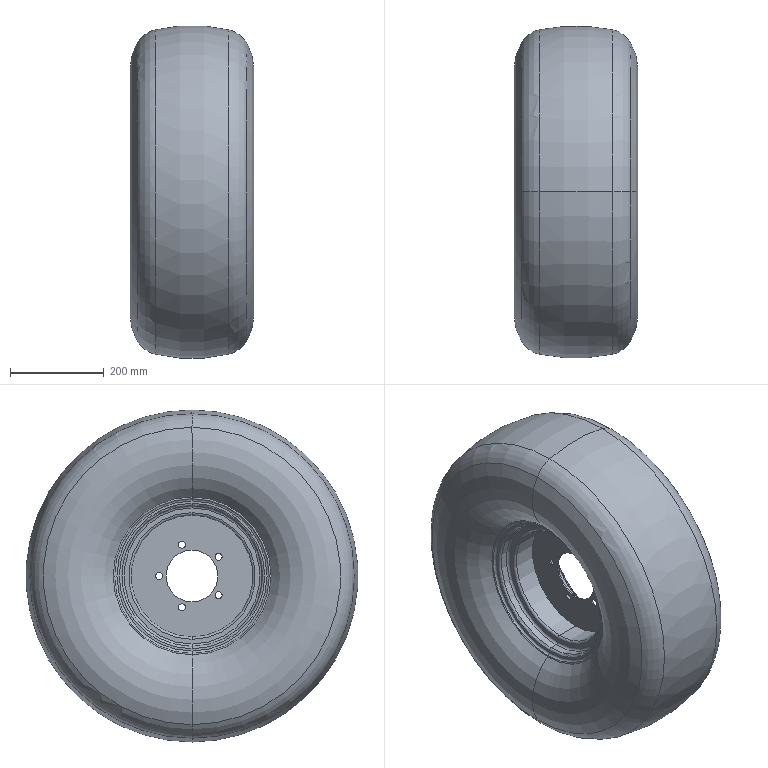Part | SolidWorks | features Revolution 2, ICE 1 | 1 solid | 56 faces | box 264 x 710 x 710 mm | volume 75274226 mm3 | torus 30 | cylinder 20 | plane 6 | commonest cylinder face diameters 15 x10 260 x4 300 x4 110 x2
STEP:
#1=CARTESIAN_POINT('',(1.5,151.631,74.074));
#2=VERTEX_POINT('',#1);
#3=CARTESIAN_POINT('',(1.5,151.631,59.074));
#4=VERTEX_POINT('',#3);
#5=CARTESIAN_POINT('',(1.5,151.631,66.574));
#6=DIRECTION('',(1.,0.,0.));
#7=DIRECTION('',(0.,0.,-1.));
#8=AXIS2_PLACEMENT_3D('',#5,#6,#7);
#9=CIRCLE('',#8,7.5);
#10=EDGE_CURVE('',#2,#4,#9,.T.);
#11=ORIENTED_EDGE('',*,*,#10,.T.);
#12=CARTESIAN_POINT('',(-1.5,151.631,59.074));
#13=VERTEX_POINT('',#12);
#14=CARTESIAN_POINT('',(1.5,151.631,59.074));
#15=DIRECTION('',(-1.,0.,0.));
#16=VECTOR('',#15,1000.);
#17=LINE('',#14,#16);
#18=EDGE_CURVE('',#4,#13,#17,.T.);
#19=ORIENTED_EDGE('',*,*,#18,.T.);
#20=CARTESIAN_POINT('',(-1.5,151.631,74.074));
#21=VERTEX_POINT('',#20);
#22=CARTESIAN_POINT('',(-1.5,151.631,66.574));
#23=DIRECTION('',(1.,0.,0.));
#24=DIRECTION('',(0.,0.,-1.));
#25=AXIS2_PLACEMENT_3D('',#22,#23,#24);
#26=CIRCLE('',#25,7.5);
#27=EDGE_CURVE('',#21,#13,#26,.T.);
#28=ORIENTED_EDGE('',*,*,#27,.F.);
#29=CARTESIAN_POINT('',(1.5,151.631,74.074));
#30=DIRECTION('',(-1.,0.,0.));
#31=VECTOR('',#30,1000.);
#32=LINE('',#29,#31);
#33=EDGE_CURVE('',#2,#21,#32,.T.);
#34=ORIENTED_EDGE('',*,*,#33,.F.);
#35=EDGE_LOOP('',(#11,#19,#28,#34));
#36=FACE_OUTER_BOUND('',#35,.T.);
#37=CARTESIAN_POINT('',(1.5,151.631,66.574));
#38=DIRECTION('',(-1.,0.,0.));
#39=DIRECTION('',(0.,0.,1.));
#40=AXIS2_PLACEMENT_3D('',#37,#38,#39);
#41=CYLINDRICAL_SURFACE('',#40,7.5);
#42=ADVANCED_FACE('',(#36),#41,.F.);
#43=CARTESIAN_POINT('',(1.5,73.369,48.645));
#44=VERTEX_POINT('',#43);
#45=CARTESIAN_POINT('',(1.5,73.369,33.645));
#46=VERTEX_POINT('',#45);
#47=CARTESIAN_POINT('',(1.5,73.369,41.145));
#48=DIRECTION('',(1.,0.,0.));
#49=DIRECTION('',(0.,0.,-1.));
#50=AXIS2_PLACEMENT_3D('',#47,#48,#49);
#51=CIRCLE('',#50,7.5);
#52=EDGE_CURVE('',#44,#46,#51,.T.);
#53=ORIENTED_EDGE('',*,*,#52,.T.);
#54=CARTESIAN_POINT('',(-1.5,73.369,33.645));
#55=VERTEX_POINT('',#54);
#56=CARTESIAN_POINT('',(1.5,73.369,33.645));
#57=DIRECTION('',(-1.,0.,0.));
#58=VECTOR('',#57,1000.);
#59=LINE('',#56,#58);
#60=EDGE_CURVE('',#46,#55,#59,.T.);
#61=ORIENTED_EDGE('',*,*,#60,.T.);
#62=CARTESIAN_POINT('',(-1.5,73.369,48.645));
#63=VERTEX_POINT('',#62);
#64=CARTESIAN_POINT('',(-1.5,73.369,41.145));
#65=DIRECTION('',(1.,0.,0.));
#66=DIRECTION('',(0.,0.,-1.));
#67=AXIS2_PLACEMENT_3D('',#64,#65,#66);
#68=CIRCLE('',#67,7.5);
#69=EDGE_CURVE('',#63,#55,#68,.T.);
#70=ORIENTED_EDGE('',*,*,#69,.F.);
#71=CARTESIAN_POINT('',(1.5,73.369,48.645));
#72=DIRECTION('',(-1.,0.,0.));
#73=VECTOR('',#72,1000.);
#74=LINE('',#71,#73);
#75=EDGE_CURVE('',#44,#63,#74,.T.);
#76=ORIENTED_EDGE('',*,*,#75,.F.);
#77=EDGE_LOOP('',(#53,#61,#70,#76));
#78=FACE_OUTER_BOUND('',#77,.T.);
#79=CARTESIAN_POINT('',(1.5,73.369,41.145));
#80=DIRECTION('',(-1.,0.,0.));
#81=DIRECTION('',(0.,0.,1.));
#82=AXIS2_PLACEMENT_3D('',#79,#80,#81);
#83=CYLINDRICAL_SURFACE('',#82,7.5);
#84=ADVANCED_FACE('',(#78),#83,.F.);
#85=CARTESIAN_POINT('',(1.5,73.369,-33.645));
#86=VERTEX_POINT('',#85);
#87=CARTESIAN_POINT('',(1.5,73.369,-48.645));
#88=VERTEX_POINT('',#87);
#89=CARTESIAN_POINT('',(1.5,73.369,-41.145));
#90=DIRECTION('',(1.,0.,0.));
#91=DIRECTION('',(0.,0.,-1.));
#92=AXIS2_PLACEMENT_3D('',#89,#90,#91);
#93=CIRCLE('',#92,7.5);
#94=EDGE_CURVE('',#86,#88,#93,.T.);
#95=ORIENTED_EDGE('',*,*,#94,.T.);
#96=CARTESIAN_POINT('',(-1.5,73.369,-48.645));
#97=VERTEX_POINT('',#96);
#98=CARTESIAN_POINT('',(1.5,73.369,-48.645));
#99=DIRECTION('',(-1.,0.,0.));
#100=VECTOR('',#99,1000.);
#101=LINE('',#98,#100);
#102=EDGE_CURVE('',#88,#97,#101,.T.);
#103=ORIENTED_EDGE('',*,*,#102,.T.);
#104=CARTESIAN_POINT('',(-1.5,73.369,-33.645));
#105=VERTEX_POINT('',#104);
#106=CARTESIAN_POINT('',(-1.5,73.369,-41.145));
#107=DIRECTION('',(1.,0.,0.));
#108=DIRECTION('',(0.,0.,-1.));
#109=AXIS2_PLACEMENT_3D('',#106,#107,#108);
#110=CIRCLE('',#109,7.5);
#111=EDGE_CURVE('',#105,#97,#110,.T.);
#112=ORIENTED_EDGE('',*,*,#111,.F.);
#113=CARTESIAN_POINT('',(1.5,73.369,-33.645));
#114=DIRECTION('',(-1.,0.,0.));
#115=VECTOR('',#114,1000.);
#116=LINE('',#113,#115);
#117=EDGE_CURVE('',#86,#105,#116,.T.);
#118=ORIENTED_EDGE('',*,*,#117,.F.);
#119=EDGE_LOOP('',(#95,#103,#112,#118));
#120=FACE_OUTER_BOUND('',#119,.T.);
#121=CARTESIAN_POINT('',(1.5,73.369,-41.145));
#122=DIRECTION('',(-1.,0.,0.));
#123=DIRECTION('',(0.,0.,1.));
#124=AXIS2_PLACEMENT_3D('',#121,#122,#123);
#125=CYLINDRICAL_SURFACE('',#124,7.5);
#126=ADVANCED_FACE('',(#120),#125,.F.);
#127=CARTESIAN_POINT('',(1.5,151.631,-59.074));
#128=VERTEX_POINT('',#127);
#129=CARTESIAN_POINT('',(1.5,151.631,-74.074));
#130=VERTEX_POINT('',#129);
#131=CARTESIAN_POINT('',(1.5,151.631,-66.574));
#132=DIRECTION('',(1.,0.,0.));
#133=DIRECTION('',(0.,0.,-1.));
#134=AXIS2_PLACEMENT_3D('',#131,#132,#133);
#135=CIRCLE('',#134,7.5);
#136=EDGE_CURVE('',#128,#130,#135,.T.);
#137=ORIENTED_EDGE('',*,*,#136,.T.);
#138=CARTESIAN_POINT('',(-1.5,151.631,-74.074));
#139=VERTEX_POINT('',#138);
#140=CARTESIAN_POINT('',(1.5,151.631,-74.074));
#141=DIRECTION('',(-1.,0.,0.));
#142=VECTOR('',#141,1000.);
#143=LINE('',#140,#142);
#144=EDGE_CURVE('',#130,#139,#143,.T.);
#145=ORIENTED_EDGE('',*,*,#144,.T.);
#146=CARTESIAN_POINT('',(-1.5,151.631,-59.074));
#147=VERTEX_POINT('',#146);
#148=CARTESIAN_POINT('',(-1.5,151.631,-66.574));
#149=DIRECTION('',(1.,0.,0.));
#150=DIRECTION('',(0.,0.,-1.));
#151=AXIS2_PLACEMENT_3D('',#148,#149,#150);
#152=CIRCLE('',#151,7.5);
#153=EDGE_CURVE('',#147,#139,#152,.T.);
#154=ORIENTED_EDGE('',*,*,#153,.F.);
#155=CARTESIAN_POINT('',(1.5,151.631,-59.074));
#156=DIRECTION('',(-1.,0.,0.));
#157=VECTOR('',#156,1000.);
#158=LINE('',#155,#157);
#159=EDGE_CURVE('',#128,#147,#158,.T.);
#160=ORIENTED_EDGE('',*,*,#159,.F.);
#161=EDGE_LOOP('',(#137,#145,#154,#160));
#162=FACE_OUTER_BOUND('',#161,.T.);
#163=CARTESIAN_POINT('',(1.5,151.631,-66.574));
#164=DIRECTION('',(-1.,0.,0.));
#165=DIRECTION('',(0.,0.,1.));
#166=AXIS2_PLACEMENT_3D('',#163,#164,#165);
#167=CYLINDRICAL_SURFACE('',#166,7.5);
#168=ADVANCED_FACE('',(#162),#167,.F.);
#169=CARTESIAN_POINT('',(1.5,200.,7.5));
#170=VERTEX_POINT('',#169);
#171=CARTESIAN_POINT('',(1.5,200.,-7.5));
#172=VERTEX_POINT('',#171);
#173=CARTESIAN_POINT('',(1.5,200.,0.));
#174=DIRECTION('',(1.,0.,0.));
#175=DIRECTION('',(0.,0.,-1.));
#176=AXIS2_PLACEMENT_3D('',#173,#174,#175);
#177=CIRCLE('',#176,7.5);
#178=EDGE_CURVE('',#170,#172,#177,.T.);
#179=ORIENTED_EDGE('',*,*,#178,.T.);
#180=CARTESIAN_POINT('',(-1.5,200.,-7.5));
#181=VERTEX_POINT('',#180);
#182=CARTESIAN_POINT('',(1.5,200.,-7.5));
#183=DIRECTION('',(-1.,0.,0.));
#184=VECTOR('',#183,1000.);
#185=LINE('',#182,#184);
#186=EDGE_CURVE('',#172,#181,#185,.T.);
#187=ORIENTED_EDGE('',*,*,#186,.T.);
#188=CARTESIAN_POINT('',(-1.5,200.,7.5));
#189=VERTEX_POINT('',#188);
#190=CARTESIAN_POINT('',(-1.5,200.,0.));
#191=DIRECTION('',(1.,0.,0.));
#192=DIRECTION('',(0.,0.,-1.));
#193=AXIS2_PLACEMENT_3D('',#190,#191,#192);
#194=CIRCLE('',#193,7.5);
#195=EDGE_CURVE('',#189,#181,#194,.T.);
#196=ORIENTED_EDGE('',*,*,#195,.F.);
#197=CARTESIAN_POINT('',(1.5,200.,7.5));
#198=DIRECTION('',(-1.,0.,0.));
#199=VECTOR('',#198,1000.);
#200=LINE('',#197,#199);
#201=EDGE_CURVE('',#170,#189,#200,.T.);
#202=ORIENTED_EDGE('',*,*,#201,.F.);
#203=EDGE_LOOP('',(#179,#187,#196,#202));
#204=FACE_OUTER_BOUND('',#203,.T.);
#205=CARTESIAN_POINT('',(1.5,200.,0.));
#206=DIRECTION('',(-1.,0.,0.));
#207=DIRECTION('',(0.,0.,1.));
#208=AXIS2_PLACEMENT_3D('',#205,#206,#207);
#209=CYLINDRICAL_SURFACE('',#208,7.5);
#210=ADVANCED_FACE('',(#204),#209,.F.);
#211=CARTESIAN_POINT('',(1.5,130.,55.));
#212=VERTEX_POINT('',#211);
#213=CARTESIAN_POINT('',(1.5,130.,-55.));
#214=VERTEX_POINT('',#213);
#215=CARTESIAN_POINT('',(1.5,130.,0.));
#216=DIRECTION('',(1.,0.,0.));
#217=DIRECTION('',(0.,0.,-1.));
#218=AXIS2_PLACEMENT_3D('',#215,#216,#217);
#219=CIRCLE('',#218,55.);
#220=EDGE_CURVE('',#212,#214,#219,.T.);
#221=ORIENTED_EDGE('',*,*,#220,.T.);
#222=CARTESIAN_POINT('',(-1.5,130.,-55.));
#223=VERTEX_POINT('',#222);
#224=CARTESIAN_POINT('',(1.5,130.,-55.));
#225=DIRECTION('',(-1.,0.,0.));
#226=VECTOR('',#225,1000.);
#227=LINE('',#224,#226);
#228=EDGE_CURVE('',#214,#223,#227,.T.);
#229=ORIENTED_EDGE('',*,*,#228,.T.);
#230=CARTESIAN_POINT('',(-1.5,130.,55.));
#231=VERTEX_POINT('',#230);
#232=CARTESIAN_POINT('',(-1.5,130.,0.));
#233=DIRECTION('',(1.,0.,0.));
#234=DIRECTION('',(0.,0.,-1.));
#235=AXIS2_PLACEMENT_3D('',#232,#233,#234);
#236=CIRCLE('',#235,55.);
#237=EDGE_CURVE('',#231,#223,#236,.T.);
#238=ORIENTED_EDGE('',*,*,#237,.F.);
#239=CARTESIAN_POINT('',(1.5,130.,55.));
#240=DIRECTION('',(-1.,0.,0.));
#241=VECTOR('',#240,1000.);
#242=LINE('',#239,#241);
#243=EDGE_CURVE('',#212,#231,#242,.T.);
#244=ORIENTED_EDGE('',*,*,#243,.F.);
#245=EDGE_LOOP('',(#221,#229,#238,#244));
#246=FACE_OUTER_BOUND('',#245,.T.);
#247=CARTESIAN_POINT('',(1.5,130.,0.));
#248=DIRECTION('',(-1.,0.,0.));
#249=DIRECTION('',(0.,0.,1.));
#250=AXIS2_PLACEMENT_3D('',#247,#248,#249);
#251=CYLINDRICAL_SURFACE('',#250,55.);
#252=ADVANCED_FACE('',(#246),#251,.F.);
#253=CARTESIAN_POINT('',(-85.,130.,-168.));
#254=VERTEX_POINT('',#253);
#255=CARTESIAN_POINT('',(-85.,130.,168.));
#256=VERTEX_POINT('',#255);
#257=CARTESIAN_POINT('',(-85.,130.,0.));
#258=DIRECTION('',(1.,0.,0.));
#259=DIRECTION('',(0.,0.,-1.));
#260=AXIS2_PLACEMENT_3D('',#257,#258,#259);
#261=CIRCLE('',#260,168.);
#262=EDGE_CURVE('',#254,#256,#261,.T.);
#263=ORIENTED_EDGE('',*,*,#262,.T.);
#264=CARTESIAN_POINT('',(-117.217,130.,316.858));
#265=VERTEX_POINT('',#264);
#266=CARTESIAN_POINT('',(-17.374,130.,260.552));
#267=DIRECTION('',(0.,1.,0.));
#268=DIRECTION('',(0.,0.,1.));
#269=AXIS2_PLACEMENT_3D('',#266,#267,#268);
#270=CIRCLE('',#269,114.626);
#271=EDGE_CURVE('',#256,#265,#270,.T.);
#272=ORIENTED_EDGE('',*,*,#271,.T.);
#273=CARTESIAN_POINT('',(-117.217,130.,-316.858));
#274=VERTEX_POINT('',#273);
#275=CARTESIAN_POINT('',(-117.217,130.,0.));
#276=DIRECTION('',(1.,0.,0.));
#277=DIRECTION('',(0.,0.,-1.));
#278=AXIS2_PLACEMENT_3D('',#275,#276,#277);
#279=CIRCLE('',#278,316.858);
#280=EDGE_CURVE('',#274,#265,#279,.T.);
#281=ORIENTED_EDGE('',*,*,#280,.F.);
#282=CARTESIAN_POINT('',(-17.374,130.,-260.552));
#283=DIRECTION('',(0.,-1.,0.));
#284=DIRECTION('',(0.,0.,-1.));
#285=AXIS2_PLACEMENT_3D('',#282,#283,#284);
#286=CIRCLE('',#285,114.626);
#287=EDGE_CURVE('',#254,#274,#286,.T.);
#288=ORIENTED_EDGE('',*,*,#287,.F.);
#289=EDGE_LOOP('',(#263,#272,#281,#288));
#290=FACE_OUTER_BOUND('',#289,.T.);
#291=CARTESIAN_POINT('',(-17.374,130.,0.));
#292=DIRECTION('',(1.,0.,0.));
#293=DIRECTION('',(0.,0.,-1.));
#294=AXIS2_PLACEMENT_3D('',#291,#292,#293);
#295=TOROIDAL_SURFACE('',#294,260.552,114.626);
#296=ADVANCED_FACE('',(#290),#295,.T.);
#297=ORIENTED_EDGE('',*,*,#280,.T.);
#298=CARTESIAN_POINT('',(-78.833,130.,345.758));
#299=VERTEX_POINT('',#298);
#300=CARTESIAN_POINT('',(-64.955,130.,287.385));
#301=DIRECTION('',(0.,1.,0.));
#302=DIRECTION('',(0.,0.,1.));
#303=AXIS2_PLACEMENT_3D('',#300,#301,#302);
#304=CIRCLE('',#303,60.);
#305=EDGE_CURVE('',#265,#299,#304,.T.);
#306=ORIENTED_EDGE('',*,*,#305,.T.);
#307=CARTESIAN_POINT('',(-78.833,130.,-345.758));
#308=VERTEX_POINT('',#307);
#309=CARTESIAN_POINT('',(-78.833,130.,0.));
#310=DIRECTION('',(1.,0.,0.));
#311=DIRECTION('',(0.,0.,-1.));
#312=AXIS2_PLACEMENT_3D('',#309,#310,#311);
#313=CIRCLE('',#312,345.758);
#314=EDGE_CURVE('',#308,#299,#313,.T.);
#315=ORIENTED_EDGE('',*,*,#314,.F.);
#316=CARTESIAN_POINT('',(-64.955,130.,-287.385));
#317=DIRECTION('',(0.,-1.,0.));
#318=DIRECTION('',(0.,0.,-1.));
#319=AXIS2_PLACEMENT_3D('',#316,#317,#318);
#320=CIRCLE('',#319,60.);
#321=EDGE_CURVE('',#274,#308,#320,.T.);
#322=ORIENTED_EDGE('',*,*,#321,.F.);
#323=EDGE_LOOP('',(#297,#306,#315,#322));
#324=FACE_OUTER_BOUND('',#323,.T.);
#325=CARTESIAN_POINT('',(-64.955,130.,0.));
#326=DIRECTION('',(1.,0.,0.));
#327=DIRECTION('',(0.,0.,-1.));
#328=AXIS2_PLACEMENT_3D('',#325,#326,#327);
#329=TOROIDAL_SURFACE('',#328,287.385,60.);
#330=ADVANCED_FACE('',(#324),#329,.T.);
#331=ORIENTED_EDGE('',*,*,#314,.T.);
#332=CARTESIAN_POINT('',(78.833,130.,345.758));
#333=VERTEX_POINT('',#332);
#334=CARTESIAN_POINT('',(0.,130.,14.167));
#335=DIRECTION('',(0.,1.,0.));
#336=DIRECTION('',(0.,0.,1.));
#337=AXIS2_PLACEMENT_3D('',#334,#335,#336);
#338=CIRCLE('',#337,340.833);
#339=EDGE_CURVE('',#299,#333,#338,.T.);
#340=ORIENTED_EDGE('',*,*,#339,.T.);
#341=CARTESIAN_POINT('',(78.833,130.,-345.758));
#342=VERTEX_POINT('',#341);
#343=CARTESIAN_POINT('',(78.833,130.,0.));
#344=DIRECTION('',(1.,0.,0.));
#345=DIRECTION('',(0.,0.,-1.));
#346=AXIS2_PLACEMENT_3D('',#343,#344,#345);
#347=CIRCLE('',#346,345.758);
#348=EDGE_CURVE('',#342,#333,#347,.T.);
#349=ORIENTED_EDGE('',*,*,#348,.F.);
#350=CARTESIAN_POINT('',(0.,130.,-14.167));
#351=DIRECTION('',(0.,-1.,0.));
#352=DIRECTION('',(0.,0.,-1.));
#353=AXIS2_PLACEMENT_3D('',#350,#351,#352);
#354=CIRCLE('',#353,340.833);
#355=EDGE_CURVE('',#308,#342,#354,.T.);
#356=ORIENTED_EDGE('',*,*,#355,.F.);
#357=EDGE_LOOP('',(#331,#340,#349,#356));
#358=FACE_OUTER_BOUND('',#357,.T.);
#359=CARTESIAN_POINT('',(0.,130.,0.));
#360=DIRECTION('',(1.,0.,0.));
#361=DIRECTION('',(0.,0.,-1.));
#362=AXIS2_PLACEMENT_3D('',#359,#360,#361);
#363=TOROIDAL_SURFACE('',#362,14.167,340.833);
#364=ADVANCED_FACE('',(#358),#363,.T.);
#365=ORIENTED_EDGE('',*,*,#348,.T.);
#366=CARTESIAN_POINT('',(117.217,130.,316.858));
#367=VERTEX_POINT('',#366);
#368=CARTESIAN_POINT('',(64.955,130.,287.385));
#369=DIRECTION('',(0.,1.,0.));
#370=DIRECTION('',(0.,0.,1.));
#371=AXIS2_PLACEMENT_3D('',#368,#369,#370);
#372=CIRCLE('',#371,60.);
#373=EDGE_CURVE('',#333,#367,#372,.T.);
#374=ORIENTED_EDGE('',*,*,#373,.T.);
#375=CARTESIAN_POINT('',(117.217,130.,-316.858));
#376=VERTEX_POINT('',#375);
#377=CARTESIAN_POINT('',(117.217,130.,0.));
#378=DIRECTION('',(1.,0.,0.));
#379=DIRECTION('',(0.,0.,-1.));
#380=AXIS2_PLACEMENT_3D('',#377,#378,#379);
#381=CIRCLE('',#380,316.858);
#382=EDGE_CURVE('',#376,#367,#381,.T.);
#383=ORIENTED_EDGE('',*,*,#382,.F.);
#384=CARTESIAN_POINT('',(64.955,130.,-287.385));
#385=DIRECTION('',(0.,-1.,0.));
#386=DIRECTION('',(0.,0.,-1.));
#387=AXIS2_PLACEMENT_3D('',#384,#385,#386);
#388=CIRCLE('',#387,60.);
#389=EDGE_CURVE('',#342,#376,#388,.T.);
#390=ORIENTED_EDGE('',*,*,#389,.F.);
#391=EDGE_LOOP('',(#365,#374,#383,#390));
#392=FACE_OUTER_BOUND('',#391,.T.);
#393=CARTESIAN_POINT('',(64.955,130.,0.));
#394=DIRECTION('',(1.,0.,0.));
#395=DIRECTION('',(0.,0.,-1.));
#396=AXIS2_PLACEMENT_3D('',#393,#394,#395);
#397=TOROIDAL_SURFACE('',#396,287.385,60.);
#398=ADVANCED_FACE('',(#392),#397,.T.);
#399=ORIENTED_EDGE('',*,*,#382,.T.);
#400=CARTESIAN_POINT('',(85.,130.,168.));
#401=VERTEX_POINT('',#400);
#402=CARTESIAN_POINT('',(17.374,130.,260.552));
#403=DIRECTION('',(0.,1.,0.));
#404=DIRECTION('',(0.,0.,1.));
#405=AXIS2_PLACEMENT_3D('',#402,#403,#404);
#406=CIRCLE('',#405,114.626);
#407=EDGE_CURVE('',#367,#401,#406,.T.);
#408=ORIENTED_EDGE('',*,*,#407,.T.);
#409=CARTESIAN_POINT('',(85.,130.,-168.));
#410=VERTEX_POINT('',#409);
#411=CARTESIAN_POINT('',(85.,130.,0.));
#412=DIRECTION('',(-1.,0.,0.));
#413=DIRECTION('',(0.,0.,1.));
#414=AXIS2_PLACEMENT_3D('',#411,#412,#413);
#415=CIRCLE('',#414,168.);
#416=EDGE_CURVE('',#401,#410,#415,.T.);
#417=ORIENTED_EDGE('',*,*,#416,.T.);
#418=CARTESIAN_POINT('',(17.374,130.,-260.552));
#419=DIRECTION('',(0.,-1.,0.));
#420=DIRECTION('',(0.,0.,-1.));
#421=AXIS2_PLACEMENT_3D('',#418,#419,#420);
#422=CIRCLE('',#421,114.626);
#423=EDGE_CURVE('',#376,#410,#422,.T.);
#424=ORIENTED_EDGE('',*,*,#423,.F.);
#425=EDGE_LOOP('',(#399,#408,#417,#424));
#426=FACE_OUTER_BOUND('',#425,.T.);
#427=CARTESIAN_POINT('',(17.374,130.,0.));
#428=DIRECTION('',(1.,0.,0.));
#429=DIRECTION('',(0.,0.,-1.));
#430=AXIS2_PLACEMENT_3D('',#427,#428,#429);
#431=TOROIDAL_SURFACE('',#430,260.552,114.626);
#432=ADVANCED_FACE('',(#426),#431,.T.);
#433=CARTESIAN_POINT('',(50.,130.,-130.));
#434=VERTEX_POINT('',#433);
#435=CARTESIAN_POINT('',(50.,130.,130.));
#436=VERTEX_POINT('',#435);
#437=CARTESIAN_POINT('',(50.,130.,0.));
#438=DIRECTION('',(-1.,0.,0.));
#439=DIRECTION('',(0.,0.,1.));
#440=AXIS2_PLACEMENT_3D('',#437,#438,#439);
#441=CIRCLE('',#440,130.);
#442=EDGE_CURVE('',#434,#436,#441,.T.);
#443=ORIENTED_EDGE('',*,*,#442,.F.);
#444=CARTESIAN_POINT('',(1.5,130.,-130.));
#445=VERTEX_POINT('',#444);
#446=CARTESIAN_POINT('',(-65.405,130.,-130.));
#447=DIRECTION('',(-1.,0.,0.));
#448=VECTOR('',#447,1000.);
#449=LINE('',#446,#448);
#450=EDGE_CURVE('',#434,#445,#449,.T.);
#451=ORIENTED_EDGE('',*,*,#450,.T.);
#452=CARTESIAN_POINT('',(1.5,130.,130.));
#453=VERTEX_POINT('',#452);
#454=CARTESIAN_POINT('',(1.5,130.,0.));
#455=DIRECTION('',(1.,0.,0.));
#456=DIRECTION('',(0.,0.,-1.));
#457=AXIS2_PLACEMENT_3D('',#454,#455,#456);
#458=CIRCLE('',#457,130.);
#459=EDGE_CURVE('',#453,#445,#458,.T.);
#460=ORIENTED_EDGE('',*,*,#459,.F.);
#461=CARTESIAN_POINT('',(-65.405,130.,130.));
#462=DIRECTION('',(-1.,0.,0.));
#463=VECTOR('',#462,1000.);
#464=LINE('',#461,#463);
#465=EDGE_CURVE('',#436,#453,#464,.T.);
#466=ORIENTED_EDGE('',*,*,#465,.F.);
#467=EDGE_LOOP('',(#443,#451,#460,#466));
#468=FACE_OUTER_BOUND('',#467,.T.);
#469=CARTESIAN_POINT('',(-65.405,130.,0.));
#470=DIRECTION('',(-1.,0.,0.));
#471=DIRECTION('',(0.,0.,1.));
#472=AXIS2_PLACEMENT_3D('',#469,#470,#471);
#473=CYLINDRICAL_SURFACE('',#472,130.);
#474=ADVANCED_FACE('',(#468),#473,.F.);
#475=CARTESIAN_POINT('',(50.,130.,0.));
#476=DIRECTION('',(-1.,0.,0.));
#477=DIRECTION('',(0.,0.,1.));
#478=AXIS2_PLACEMENT_3D('',#475,#476,#477);
#479=CIRCLE('',#478,130.);
#480=EDGE_CURVE('',#436,#434,#479,.T.);
#481=ORIENTED_EDGE('',*,*,#480,.T.);
#482=CARTESIAN_POINT('',(55.,130.,-135.));
#483=VERTEX_POINT('',#482);
#484=CARTESIAN_POINT('',(50.,130.,-135.));
#485=DIRECTION('',(0.,1.,0.));
#486=DIRECTION('',(0.,0.,1.));
#487=AXIS2_PLACEMENT_3D('',#484,#485,#486);
#488=CIRCLE('',#487,5.);
#489=EDGE_CURVE('',#434,#483,#488,.T.);
#490=ORIENTED_EDGE('',*,*,#489,.T.);
#491=CARTESIAN_POINT('',(55.,130.,135.));
#492=VERTEX_POINT('',#491);
#493=CARTESIAN_POINT('',(55.,130.,0.));
#494=DIRECTION('',(-1.,0.,0.));
#495=DIRECTION('',(0.,0.,1.));
#496=AXIS2_PLACEMENT_3D('',#493,#494,#495);
#497=CIRCLE('',#496,135.);
#498=EDGE_CURVE('',#492,#483,#497,.T.);
#499=ORIENTED_EDGE('',*,*,#498,.F.);
#500=CARTESIAN_POINT('',(50.,130.,135.));
#501=DIRECTION('',(0.,-1.,0.));
#502=DIRECTION('',(0.,0.,-1.));
#503=AXIS2_PLACEMENT_3D('',#500,#501,#502);
#504=CIRCLE('',#503,5.);
#505=EDGE_CURVE('',#436,#492,#504,.T.);
#506=ORIENTED_EDGE('',*,*,#505,.F.);
#507=EDGE_LOOP('',(#481,#490,#499,#506));
#508=FACE_OUTER_BOUND('',#507,.T.);
#509=CARTESIAN_POINT('',(50.,130.,0.));
#510=DIRECTION('',(-1.,0.,0.));
#511=DIRECTION('',(0.,0.,1.));
#512=AXIS2_PLACEMENT_3D('',#509,#510,#511);
#513=TOROIDAL_SURFACE('',#512,135.,5.);
#514=ADVANCED_FACE('',(#508),#513,.T.);
#515=CARTESIAN_POINT('',(60.,130.,-150.));
#516=VERTEX_POINT('',#515);
#517=CARTESIAN_POINT('',(60.,130.,150.));
#518=VERTEX_POINT('',#517);
#519=CARTESIAN_POINT('',(60.,130.,0.));
#520=DIRECTION('',(-1.,0.,0.));
#521=DIRECTION('',(0.,0.,1.));
#522=AXIS2_PLACEMENT_3D('',#519,#520,#521);
#523=CIRCLE('',#522,150.);
#524=EDGE_CURVE('',#516,#518,#523,.T.);
#525=ORIENTED_EDGE('',*,*,#524,.F.);
#526=CARTESIAN_POINT('',(55.,130.,-145.));
#527=VERTEX_POINT('',#526);
#528=CARTESIAN_POINT('',(60.,130.,-145.));
#529=DIRECTION('',(0.,1.,0.));
#530=DIRECTION('',(0.,0.,1.));
#531=AXIS2_PLACEMENT_3D('',#528,#529,#530);
#532=CIRCLE('',#531,5.);
#533=EDGE_CURVE('',#516,#527,#532,.T.);
#534=ORIENTED_EDGE('',*,*,#533,.T.);
#535=CARTESIAN_POINT('',(55.,130.,145.));
#536=VERTEX_POINT('',#535);
#537=CARTESIAN_POINT('',(55.,130.,0.));
#538=DIRECTION('',(-1.,0.,0.));
#539=DIRECTION('',(0.,0.,1.));
#540=AXIS2_PLACEMENT_3D('',#537,#538,#539);
#541=CIRCLE('',#540,145.);
#542=EDGE_CURVE('',#527,#536,#541,.T.);
#543=ORIENTED_EDGE('',*,*,#542,.T.);
#544=CARTESIAN_POINT('',(60.,130.,145.));
#545=DIRECTION('',(0.,-1.,0.));
#546=DIRECTION('',(0.,0.,-1.));
#547=AXIS2_PLACEMENT_3D('',#544,#545,#546);
#548=CIRCLE('',#547,5.);
#549=EDGE_CURVE('',#518,#536,#548,.T.);
#550=ORIENTED_EDGE('',*,*,#549,.F.);
#551=EDGE_LOOP('',(#525,#534,#543,#550));
#552=FACE_OUTER_BOUND('',#551,.T.);
#553=CARTESIAN_POINT('',(60.,130.,0.));
#554=DIRECTION('',(-1.,0.,0.));
#555=DIRECTION('',(0.,0.,1.));
#556=AXIS2_PLACEMENT_3D('',#553,#554,#555);
#557=TOROIDAL_SURFACE('',#556,145.,5.);
#558=ADVANCED_FACE('',(#552),#557,.F.);
#559=CARTESIAN_POINT('',(75.,130.,-150.));
#560=VERTEX_POINT('',#559);
#561=CARTESIAN_POINT('',(75.,130.,150.));
#562=VERTEX_POINT('',#561);
#563=CARTESIAN_POINT('',(75.,130.,0.));
#564=DIRECTION('',(-1.,0.,0.));
#565=DIRECTION('',(0.,0.,1.));
#566=AXIS2_PLACEMENT_3D('',#563,#564,#565);
#567=CIRCLE('',#566,150.);
#568=EDGE_CURVE('',#560,#562,#567,.T.);
#569=ORIENTED_EDGE('',*,*,#568,.F.);
#570=CARTESIAN_POINT('',(-65.405,130.,-150.));
#571=DIRECTION('',(-1.,0.,0.));
#572=VECTOR('',#571,1000.);
#573=LINE('',#570,#572);
#574=EDGE_CURVE('',#560,#516,#573,.T.);
#575=ORIENTED_EDGE('',*,*,#574,.T.);
#576=ORIENTED_EDGE('',*,*,#524,.T.);
#577=CARTESIAN_POINT('',(-65.405,130.,150.));
#578=DIRECTION('',(-1.,0.,0.));
#579=VECTOR('',#578,1000.);
#580=LINE('',#577,#579);
#581=EDGE_CURVE('',#562,#518,#580,.T.);
#582=ORIENTED_EDGE('',*,*,#581,.F.);
#583=EDGE_LOOP('',(#569,#575,#576,#582));
#584=FACE_OUTER_BOUND('',#583,.T.);
#585=CARTESIAN_POINT('',(-65.405,130.,0.));
#586=DIRECTION('',(-1.,0.,0.));
#587=DIRECTION('',(0.,0.,1.));
#588=AXIS2_PLACEMENT_3D('',#585,#586,#587);
#589=CYLINDRICAL_SURFACE('',#588,150.);
#590=ADVANCED_FACE('',(#584),#589,.F.);
#591=CARTESIAN_POINT('',(75.,130.,0.));
#592=DIRECTION('',(-1.,0.,0.));
#593=DIRECTION('',(0.,0.,1.));
#594=AXIS2_PLACEMENT_3D('',#591,#592,#593);
#595=CIRCLE('',#594,150.);
#596=EDGE_CURVE('',#562,#560,#595,.T.);
#597=ORIENTED_EDGE('',*,*,#596,.T.);
#598=CARTESIAN_POINT('',(80.,130.,-155.));
#599=VERTEX_POINT('',#598);
#600=CARTESIAN_POINT('',(75.,130.,-155.));
#601=DIRECTION('',(0.,1.,0.));
#602=DIRECTION('',(0.,0.,1.));
#603=AXIS2_PLACEMENT_3D('',#600,#601,#602);
#604=CIRCLE('',#603,5.);
#605=EDGE_CURVE('',#560,#599,#604,.T.);
#606=ORIENTED_EDGE('',*,*,#605,.T.);
#607=CARTESIAN_POINT('',(80.,130.,155.));
#608=VERTEX_POINT('',#607);
#609=CARTESIAN_POINT('',(80.,130.,0.));
#610=DIRECTION('',(-1.,0.,0.));
#611=DIRECTION('',(0.,0.,1.));
#612=AXIS2_PLACEMENT_3D('',#609,#610,#611);
#613=CIRCLE('',#612,155.);
#614=EDGE_CURVE('',#608,#599,#613,.T.);
#615=ORIENTED_EDGE('',*,*,#614,.F.);
#616=CARTESIAN_POINT('',(75.,130.,155.));
#617=DIRECTION('',(0.,-1.,0.));
#618=DIRECTION('',(0.,0.,-1.));
#619=AXIS2_PLACEMENT_3D('',#616,#617,#618);
#620=CIRCLE('',#619,5.);
#621=EDGE_CURVE('',#562,#608,#620,.T.);
#622=ORIENTED_EDGE('',*,*,#621,.F.);
#623=EDGE_LOOP('',(#597,#606,#615,#622));
#624=FACE_OUTER_BOUND('',#623,.T.);
#625=CARTESIAN_POINT('',(75.,130.,0.));
#626=DIRECTION('',(-1.,0.,0.));
#627=DIRECTION('',(0.,0.,1.));
#628=AXIS2_PLACEMENT_3D('',#625,#626,#627);
#629=TOROIDAL_SURFACE('',#628,155.,5.);
#630=ADVANCED_FACE('',(#624),#629,.T.);
#631=CARTESIAN_POINT('',(85.,130.,-165.));
#632=VERTEX_POINT('',#631);
#633=CARTESIAN_POINT('',(85.,130.,165.));
#634=VERTEX_POINT('',#633);
#635=CARTESIAN_POINT('',(85.,130.,0.));
#636=DIRECTION('',(-1.,0.,0.));
#637=DIRECTION('',(0.,0.,1.));
#638=AXIS2_PLACEMENT_3D('',#635,#636,#637);
#639=CIRCLE('',#638,165.);
#640=EDGE_CURVE('',#632,#634,#639,.T.);
#641=ORIENTED_EDGE('',*,*,#640,.F.);
#642=CARTESIAN_POINT('',(80.,130.,-160.));
#643=VERTEX_POINT('',#642);
#644=CARTESIAN_POINT('',(85.,130.,-160.));
#645=DIRECTION('',(0.,1.,0.));
#646=DIRECTION('',(0.,0.,1.));
#647=AXIS2_PLACEMENT_3D('',#644,#645,#646);
#648=CIRCLE('',#647,5.);
#649=EDGE_CURVE('',#632,#643,#648,.T.);
#650=ORIENTED_EDGE('',*,*,#649,.T.);
#651=CARTESIAN_POINT('',(80.,130.,160.));
#652=VERTEX_POINT('',#651);
#653=CARTESIAN_POINT('',(80.,130.,0.));
#654=DIRECTION('',(-1.,0.,0.));
#655=DIRECTION('',(0.,0.,1.));
#656=AXIS2_PLACEMENT_3D('',#653,#654,#655);
#657=CIRCLE('',#656,160.);
#658=EDGE_CURVE('',#643,#652,#657,.T.);
#659=ORIENTED_EDGE('',*,*,#658,.T.);
#660=CARTESIAN_POINT('',(85.,130.,160.));
#661=DIRECTION('',(0.,-1.,0.));
#662=DIRECTION('',(0.,0.,-1.));
#663=AXIS2_PLACEMENT_3D('',#660,#661,#662);
#664=CIRCLE('',#663,5.);
#665=EDGE_CURVE('',#634,#652,#664,.T.);
#666=ORIENTED_EDGE('',*,*,#665,.F.);
#667=EDGE_LOOP('',(#641,#650,#659,#666));
#668=FACE_OUTER_BOUND('',#667,.T.);
#669=CARTESIAN_POINT('',(85.,130.,0.));
#670=DIRECTION('',(-1.,0.,0.));
#671=DIRECTION('',(0.,0.,1.));
#672=AXIS2_PLACEMENT_3D('',#669,#670,#671);
#673=TOROIDAL_SURFACE('',#672,160.,5.);
#674=ADVANCED_FACE('',(#668),#673,.F.);
#675=CARTESIAN_POINT('',(85.,130.,0.));
#676=DIRECTION('',(-1.,0.,0.));
#677=DIRECTION('',(0.,0.,1.));
#678=AXIS2_PLACEMENT_3D('',#675,#676,#677);
#679=CIRCLE('',#678,165.);
#680=EDGE_CURVE('',#634,#632,#679,.T.);
#681=ORIENTED_EDGE('',*,*,#680,.T.);
#682=CARTESIAN_POINT('',(85.,130.,-166.5));
#683=DIRECTION('',(0.,1.,0.));
#684=DIRECTION('',(0.,0.,1.));
#685=AXIS2_PLACEMENT_3D('',#682,#683,#684);
#686=CIRCLE('',#685,1.5);
#687=EDGE_CURVE('',#632,#410,#686,.T.);
#688=ORIENTED_EDGE('',*,*,#687,.T.);
#689=ORIENTED_EDGE('',*,*,#416,.F.);
#690=CARTESIAN_POINT('',(85.,130.,166.5));
#691=DIRECTION('',(0.,-1.,0.));
#692=DIRECTION('',(0.,0.,-1.));
#693=AXIS2_PLACEMENT_3D('',#690,#691,#692);
#694=CIRCLE('',#693,1.5);
#695=EDGE_CURVE('',#634,#401,#694,.T.);
#696=ORIENTED_EDGE('',*,*,#695,.F.);
#697=EDGE_LOOP('',(#681,#688,#689,#696));
#698=FACE_OUTER_BOUND('',#697,.T.);
#699=CARTESIAN_POINT('',(85.,130.,0.));
#700=DIRECTION('',(-1.,0.,0.));
#701=DIRECTION('',(0.,0.,1.));
#702=AXIS2_PLACEMENT_3D('',#699,#700,#701);
#703=TOROIDAL_SURFACE('',#702,166.5,1.5);
#704=ADVANCED_FACE('',(#698),#703,.T.);
#705=ORIENTED_EDGE('',*,*,#262,.F.);
#706=CARTESIAN_POINT('',(-85.,130.,-165.));
#707=VERTEX_POINT('',#706);
#708=CARTESIAN_POINT('',(-85.,130.,-166.5));
#709=DIRECTION('',(0.,1.,0.));
#710=DIRECTION('',(0.,0.,1.));
#711=AXIS2_PLACEMENT_3D('',#708,#709,#710);
#712=CIRCLE('',#711,1.5);
#713=EDGE_CURVE('',#254,#707,#712,.T.);
#714=ORIENTED_EDGE('',*,*,#713,.T.);
#715=CARTESIAN_POINT('',(-85.,130.,165.));
#716=VERTEX_POINT('',#715);
#717=CARTESIAN_POINT('',(-85.,130.,0.));
#718=DIRECTION('',(-1.,0.,0.));
#719=DIRECTION('',(0.,0.,1.));
#720=AXIS2_PLACEMENT_3D('',#717,#718,#719);
#721=CIRCLE('',#720,165.);
#722=EDGE_CURVE('',#716,#707,#721,.T.);
#723=ORIENTED_EDGE('',*,*,#722,.F.);
#724=CARTESIAN_POINT('',(-85.,130.,166.5));
#725=DIRECTION('',(0.,-1.,0.));
#726=DIRECTION('',(0.,0.,-1.));
#727=AXIS2_PLACEMENT_3D('',#724,#725,#726);
#728=CIRCLE('',#727,1.5);
#729=EDGE_CURVE('',#256,#716,#728,.T.);
#730=ORIENTED_EDGE('',*,*,#729,.F.);
#731=EDGE_LOOP('',(#705,#714,#723,#730));
#732=FACE_OUTER_BOUND('',#731,.T.);
#733=CARTESIAN_POINT('',(-85.,130.,0.));
#734=DIRECTION('',(-1.,0.,0.));
#735=DIRECTION('',(0.,0.,1.));
#736=AXIS2_PLACEMENT_3D('',#733,#734,#735);
#737=TOROIDAL_SURFACE('',#736,166.5,1.5);
#738=ADVANCED_FACE('',(#732),#737,.T.);
#739=CARTESIAN_POINT('',(-80.,130.,-160.));
#740=VERTEX_POINT('',#739);
#741=CARTESIAN_POINT('',(-80.,130.,160.));
#742=VERTEX_POINT('',#741);
#743=CARTESIAN_POINT('',(-80.,130.,0.));
#744=DIRECTION('',(-1.,0.,0.));
#745=DIRECTION('',(0.,0.,1.));
#746=AXIS2_PLACEMENT_3D('',#743,#744,#745);
#747=CIRCLE('',#746,160.);
#748=EDGE_CURVE('',#740,#742,#747,.T.);
#749=ORIENTED_EDGE('',*,*,#748,.F.);
#750=CARTESIAN_POINT('',(-85.,130.,-160.));
#751=DIRECTION('',(0.,1.,0.));
#752=DIRECTION('',(0.,0.,1.));
#753=AXIS2_PLACEMENT_3D('',#750,#751,#752);
#754=CIRCLE('',#753,5.);
#755=EDGE_CURVE('',#740,#707,#754,.T.);
#756=ORIENTED_EDGE('',*,*,#755,.T.);
#757=CARTESIAN_POINT('',(-85.,130.,0.));
#758=DIRECTION('',(-1.,0.,0.));
#759=DIRECTION('',(0.,0.,1.));
#760=AXIS2_PLACEMENT_3D('',#757,#758,#759);
#761=CIRCLE('',#760,165.);
#762=EDGE_CURVE('',#707,#716,#761,.T.);
#763=ORIENTED_EDGE('',*,*,#762,.T.);
#764=CARTESIAN_POINT('',(-85.,130.,160.));
#765=DIRECTION('',(0.,-1.,0.));
#766=DIRECTION('',(0.,0.,-1.));
#767=AXIS2_PLACEMENT_3D('',#764,#765,#766);
#768=CIRCLE('',#767,5.);
#769=EDGE_CURVE('',#742,#716,#768,.T.);
#770=ORIENTED_EDGE('',*,*,#769,.F.);
#771=EDGE_LOOP('',(#749,#756,#763,#770));
#772=FACE_OUTER_BOUND('',#771,.T.);
#773=CARTESIAN_POINT('',(-85.,130.,0.));
#774=DIRECTION('',(-1.,0.,0.));
#775=DIRECTION('',(0.,0.,1.));
#776=AXIS2_PLACEMENT_3D('',#773,#774,#775);
#777=TOROIDAL_SURFACE('',#776,160.,5.);
#778=ADVANCED_FACE('',(#772),#777,.F.);
#779=CARTESIAN_POINT('',(-80.,130.,155.));
#780=VERTEX_POINT('',#779);
#781=CARTESIAN_POINT('',(-80.,130.,-155.));
#782=VERTEX_POINT('',#781);
#783=CARTESIAN_POINT('',(-80.,130.,0.));
#784=DIRECTION('',(-1.,0.,0.));
#785=DIRECTION('',(0.,0.,1.));
#786=AXIS2_PLACEMENT_3D('',#783,#784,#785);
#787=CIRCLE('',#786,155.);
#788=EDGE_CURVE('',#780,#782,#787,.T.);
#789=ORIENTED_EDGE('',*,*,#788,.T.);
#790=CARTESIAN_POINT('',(-75.,130.,-150.));
#791=VERTEX_POINT('',#790);
#792=CARTESIAN_POINT('',(-75.,130.,-155.));
#793=DIRECTION('',(0.,1.,0.));
#794=DIRECTION('',(0.,0.,1.));
#795=AXIS2_PLACEMENT_3D('',#792,#793,#794);
#796=CIRCLE('',#795,5.);
#797=EDGE_CURVE('',#782,#791,#796,.T.);
#798=ORIENTED_EDGE('',*,*,#797,.T.);
#799=CARTESIAN_POINT('',(-75.,130.,150.));
#800=VERTEX_POINT('',#799);
#801=CARTESIAN_POINT('',(-75.,130.,0.));
#802=DIRECTION('',(-1.,0.,0.));
#803=DIRECTION('',(0.,0.,1.));
#804=AXIS2_PLACEMENT_3D('',#801,#802,#803);
#805=CIRCLE('',#804,150.);
#806=EDGE_CURVE('',#800,#791,#805,.T.);
#807=ORIENTED_EDGE('',*,*,#806,.F.);
#808=CARTESIAN_POINT('',(-75.,130.,155.));
#809=DIRECTION('',(0.,-1.,0.));
#810=DIRECTION('',(0.,0.,-1.));
#811=AXIS2_PLACEMENT_3D('',#808,#809,#810);
#812=CIRCLE('',#811,5.);
#813=EDGE_CURVE('',#780,#800,#812,.T.);
#814=ORIENTED_EDGE('',*,*,#813,.F.);
#815=EDGE_LOOP('',(#789,#798,#807,#814));
#816=FACE_OUTER_BOUND('',#815,.T.);
#817=CARTESIAN_POINT('',(-75.,130.,0.));
#818=DIRECTION('',(-1.,0.,0.));
#819=DIRECTION('',(0.,0.,1.));
#820=AXIS2_PLACEMENT_3D('',#817,#818,#819);
#821=TOROIDAL_SURFACE('',#820,155.,5.);
#822=ADVANCED_FACE('',(#816),#821,.T.);
#823=CARTESIAN_POINT('',(-60.,130.,-150.));
#824=VERTEX_POINT('',#823);
#825=CARTESIAN_POINT('',(-60.,130.,150.));
#826=VERTEX_POINT('',#825);
#827=CARTESIAN_POINT('',(-60.,130.,0.));
#828=DIRECTION('',(-1.,0.,0.));
#829=DIRECTION('',(0.,0.,1.));
#830=AXIS2_PLACEMENT_3D('',#827,#828,#829);
#831=CIRCLE('',#830,150.);
#832=EDGE_CURVE('',#824,#826,#831,.T.);
#833=ORIENTED_EDGE('',*,*,#832,.F.);
#834=CARTESIAN_POINT('',(-65.405,130.,-150.));
#835=DIRECTION('',(-1.,0.,0.));
#836=VECTOR('',#835,1000.);
#837=LINE('',#834,#836);
#838=EDGE_CURVE('',#824,#791,#837,.T.);
#839=ORIENTED_EDGE('',*,*,#838,.T.);
#840=CARTESIAN_POINT('',(-75.,130.,0.));
#841=DIRECTION('',(-1.,0.,0.));
#842=DIRECTION('',(0.,0.,1.));
#843=AXIS2_PLACEMENT_3D('',#840,#841,#842);
#844=CIRCLE('',#843,150.);
#845=EDGE_CURVE('',#791,#800,#844,.T.);
#846=ORIENTED_EDGE('',*,*,#845,.T.);
#847=CARTESIAN_POINT('',(-65.405,130.,150.));
#848=DIRECTION('',(-1.,0.,0.));
#849=VECTOR('',#848,1000.);
#850=LINE('',#847,#849);
#851=EDGE_CURVE('',#826,#800,#850,.T.);
#852=ORIENTED_EDGE('',*,*,#851,.F.);
#853=EDGE_LOOP('',(#833,#839,#846,#852));
#854=FACE_OUTER_BOUND('',#853,.T.);
#855=CARTESIAN_POINT('',(-65.405,130.,0.));
#856=DIRECTION('',(-1.,0.,0.));
#857=DIRECTION('',(0.,0.,1.));
#858=AXIS2_PLACEMENT_3D('',#855,#856,#857);
#859=CYLINDRICAL_SURFACE('',#858,150.);
#860=ADVANCED_FACE('',(#854),#859,.F.);
#861=CARTESIAN_POINT('',(-55.,130.,-145.));
#862=VERTEX_POINT('',#861);
#863=CARTESIAN_POINT('',(-55.,130.,145.));
#864=VERTEX_POINT('',#863);
#865=CARTESIAN_POINT('',(-55.,130.,0.));
#866=DIRECTION('',(-1.,0.,0.));
#867=DIRECTION('',(0.,0.,1.));
#868=AXIS2_PLACEMENT_3D('',#865,#866,#867);
#869=CIRCLE('',#868,145.);
#870=EDGE_CURVE('',#862,#864,#869,.T.);
#871=ORIENTED_EDGE('',*,*,#870,.F.);
#872=CARTESIAN_POINT('',(-60.,130.,-145.));
#873=DIRECTION('',(0.,1.,0.));
#874=DIRECTION('',(0.,0.,1.));
#875=AXIS2_PLACEMENT_3D('',#872,#873,#874);
#876=CIRCLE('',#875,5.);
#877=EDGE_CURVE('',#862,#824,#876,.T.);
#878=ORIENTED_EDGE('',*,*,#877,.T.);
#879=ORIENTED_EDGE('',*,*,#832,.T.);
#880=CARTESIAN_POINT('',(-60.,130.,145.));
#881=DIRECTION('',(0.,-1.,0.));
#882=DIRECTION('',(0.,0.,-1.));
#883=AXIS2_PLACEMENT_3D('',#880,#881,#882);
#884=CIRCLE('',#883,5.);
#885=EDGE_CURVE('',#864,#826,#884,.T.);
#886=ORIENTED_EDGE('',*,*,#885,.F.);
#887=EDGE_LOOP('',(#871,#878,#879,#886));
#888=FACE_OUTER_BOUND('',#887,.T.);
#889=CARTESIAN_POINT('',(-60.,130.,0.));
#890=DIRECTION('',(-1.,0.,0.));
#891=DIRECTION('',(0.,0.,1.));
#892=AXIS2_PLACEMENT_3D('',#889,#890,#891);
#893=TOROIDAL_SURFACE('',#892,145.,5.);
#894=ADVANCED_FACE('',(#888),#893,.F.);
#895=CARTESIAN_POINT('',(-55.,130.,135.));
#896=VERTEX_POINT('',#895);
#897=CARTESIAN_POINT('',(-55.,130.,-135.));
#898=VERTEX_POINT('',#897);
#899=CARTESIAN_POINT('',(-55.,130.,0.));
#900=DIRECTION('',(-1.,0.,0.));
#901=DIRECTION('',(0.,0.,1.));
#902=AXIS2_PLACEMENT_3D('',#899,#900,#901);
#903=CIRCLE('',#902,135.);
#904=EDGE_CURVE('',#896,#898,#903,.T.);
#905=ORIENTED_EDGE('',*,*,#904,.T.);
#906=CARTESIAN_POINT('',(-50.,130.,-130.));
#907=VERTEX_POINT('',#906);
#908=CARTESIAN_POINT('',(-50.,130.,-135.));
#909=DIRECTION('',(0.,1.,0.));
#910=DIRECTION('',(0.,0.,1.));
#911=AXIS2_PLACEMENT_3D('',#908,#909,#910);
#912=CIRCLE('',#911,5.);
#913=EDGE_CURVE('',#898,#907,#912,.T.);
#914=ORIENTED_EDGE('',*,*,#913,.T.);
#915=CARTESIAN_POINT('',(-50.,130.,130.));
#916=VERTEX_POINT('',#915);
#917=CARTESIAN_POINT('',(-50.,130.,0.));
#918=DIRECTION('',(-1.,0.,0.));
#919=DIRECTION('',(0.,0.,1.));
#920=AXIS2_PLACEMENT_3D('',#917,#918,#919);
#921=CIRCLE('',#920,130.);
#922=EDGE_CURVE('',#916,#907,#921,.T.);
#923=ORIENTED_EDGE('',*,*,#922,.F.);
#924=CARTESIAN_POINT('',(-50.,130.,135.));
#925=DIRECTION('',(0.,-1.,0.));
#926=DIRECTION('',(0.,0.,-1.));
#927=AXIS2_PLACEMENT_3D('',#924,#925,#926);
#928=CIRCLE('',#927,5.);
#929=EDGE_CURVE('',#896,#916,#928,.T.);
#930=ORIENTED_EDGE('',*,*,#929,.F.);
#931=EDGE_LOOP('',(#905,#914,#923,#930));
#932=FACE_OUTER_BOUND('',#931,.T.);
#933=CARTESIAN_POINT('',(-50.,130.,0.));
#934=DIRECTION('',(-1.,0.,0.));
#935=DIRECTION('',(0.,0.,1.));
#936=AXIS2_PLACEMENT_3D('',#933,#934,#935);
#937=TOROIDAL_SURFACE('',#936,135.,5.);
#938=ADVANCED_FACE('',(#932),#937,.T.);
#939=CARTESIAN_POINT('',(-1.5,130.,130.));
#940=VERTEX_POINT('',#939);
#941=CARTESIAN_POINT('',(-1.5,130.,-130.));
#942=VERTEX_POINT('',#941);
#943=CARTESIAN_POINT('',(-1.5,130.,0.));
#944=DIRECTION('',(1.,0.,0.));
#945=DIRECTION('',(0.,0.,-1.));
#946=AXIS2_PLACEMENT_3D('',#943,#944,#945);
#947=CIRCLE('',#946,130.);
#948=EDGE_CURVE('',#940,#942,#947,.T.);
#949=ORIENTED_EDGE('',*,*,#948,.T.);
#950=CARTESIAN_POINT('',(-65.405,130.,-130.));
#951=DIRECTION('',(-1.,0.,0.));
#952=VECTOR('',#951,1000.);
#953=LINE('',#950,#952);
#954=EDGE_CURVE('',#942,#907,#953,.T.);
#955=ORIENTED_EDGE('',*,*,#954,.T.);
#956=CARTESIAN_POINT('',(-50.,130.,0.));
#957=DIRECTION('',(-1.,0.,0.));
#958=DIRECTION('',(0.,0.,1.));
#959=AXIS2_PLACEMENT_3D('',#956,#957,#958);
#960=CIRCLE('',#959,130.);
#961=EDGE_CURVE('',#907,#916,#960,.T.);
#962=ORIENTED_EDGE('',*,*,#961,.T.);
#963=CARTESIAN_POINT('',(-65.405,130.,130.));
#964=DIRECTION('',(-1.,0.,0.));
#965=VECTOR('',#964,1000.);
#966=LINE('',#963,#965);
#967=EDGE_CURVE('',#940,#916,#966,.T.);
#968=ORIENTED_EDGE('',*,*,#967,.F.);
#969=EDGE_LOOP('',(#949,#955,#962,#968));
#970=FACE_OUTER_BOUND('',#969,.T.);
#971=CARTESIAN_POINT('',(-65.405,130.,0.));
#972=DIRECTION('',(-1.,0.,0.));
#973=DIRECTION('',(0.,0.,1.));
#974=AXIS2_PLACEMENT_3D('',#971,#972,#973);
#975=CYLINDRICAL_SURFACE('',#974,130.);
#976=ADVANCED_FACE('',(#970),#975,.F.);
#977=ORIENTED_EDGE('',*,*,#954,.F.);
#978=CARTESIAN_POINT('',(-1.5,130.,0.));
#979=DIRECTION('',(1.,0.,0.));
#980=DIRECTION('',(0.,0.,-1.));
#981=AXIS2_PLACEMENT_3D('',#978,#979,#980);
#982=CIRCLE('',#981,130.);
#983=EDGE_CURVE('',#942,#940,#982,.T.);
#984=ORIENTED_EDGE('',*,*,#983,.T.);
#985=ORIENTED_EDGE('',*,*,#967,.T.);
#986=ORIENTED_EDGE('',*,*,#922,.T.);
#987=EDGE_LOOP('',(#977,#984,#985,#986));
#988=FACE_OUTER_BOUND('',#987,.T.);
#989=CARTESIAN_POINT('',(-65.405,130.,0.));
#990=DIRECTION('',(-1.,0.,0.));
#991=DIRECTION('',(0.,0.,1.));
#992=AXIS2_PLACEMENT_3D('',#989,#990,#991);
#993=CYLINDRICAL_SURFACE('',#992,130.);
#994=ADVANCED_FACE('',(#988),#993,.F.);
#995=ORIENTED_EDGE('',*,*,#913,.F.);
#996=CARTESIAN_POINT('',(-55.,130.,0.));
#997=DIRECTION('',(-1.,0.,0.));
#998=DIRECTION('',(0.,0.,1.));
#999=AXIS2_PLACEMENT_3D('',#996,#997,#998);
#1000=CIRCLE('',#999,135.);
#1001=EDGE_CURVE('',#898,#896,#1000,.T.);
#1002=ORIENTED_EDGE('',*,*,#1001,.T.);
#1003=ORIENTED_EDGE('',*,*,#929,.T.);
#1004=ORIENTED_EDGE('',*,*,#961,.F.);
#1005=EDGE_LOOP('',(#995,#1002,#1003,#1004));
#1006=FACE_OUTER_BOUND('',#1005,.T.);
#1007=CARTESIAN_POINT('',(-50.,130.,0.));
#1008=DIRECTION('',(-1.,0.,0.));
#1009=DIRECTION('',(0.,0.,1.));
#1010=AXIS2_PLACEMENT_3D('',#1007,#1008,#1009);
#1011=TOROIDAL_SURFACE('',#1010,135.,5.);
#1012=ADVANCED_FACE('',(#1006),#1011,.T.);
#1013=CARTESIAN_POINT('',(-55.,130.,0.));
#1014=DIRECTION('',(-1.,0.,0.));
#1015=DIRECTION('',(0.,0.,1.));
#1016=AXIS2_PLACEMENT_3D('',#1013,#1014,#1015);
#1017=CIRCLE('',#1016,145.);
#1018=EDGE_CURVE('',#864,#862,#1017,.T.);
#1019=ORIENTED_EDGE('',*,*,#1018,.T.);
#1020=ORIENTED_EDGE('',*,*,#870,.T.);
#1021=EDGE_LOOP('',(#1019,#1020));
#1022=FACE_OUTER_BOUND('',#1021,.T.);
#1023=ORIENTED_EDGE('',*,*,#904,.F.);
#1024=ORIENTED_EDGE('',*,*,#1001,.F.);
#1025=EDGE_LOOP('',(#1023,#1024));
#1026=FACE_BOUND('',#1025,.T.);
#1027=CARTESIAN_POINT('',(-55.,-5.,0.));
#1028=DIRECTION('',(-1.,0.,0.));
#1029=DIRECTION('',(0.,0.,1.));
#1030=AXIS2_PLACEMENT_3D('',#1027,#1028,#1029);
#1031=PLANE('',#1030);
#1032=ADVANCED_FACE('',(#1022,#1026),#1031,.T.);
#1033=ORIENTED_EDGE('',*,*,#877,.F.);
#1034=ORIENTED_EDGE('',*,*,#1018,.F.);
#1035=ORIENTED_EDGE('',*,*,#885,.T.);
#1036=CARTESIAN_POINT('',(-60.,130.,0.));
#1037=DIRECTION('',(-1.,0.,0.));
#1038=DIRECTION('',(0.,0.,1.));
#1039=AXIS2_PLACEMENT_3D('',#1036,#1037,#1038);
#1040=CIRCLE('',#1039,150.);
#1041=EDGE_CURVE('',#826,#824,#1040,.T.);
#1042=ORIENTED_EDGE('',*,*,#1041,.T.);
#1043=EDGE_LOOP('',(#1033,#1034,#1035,#1042));
#1044=FACE_OUTER_BOUND('',#1043,.T.);
#1045=CARTESIAN_POINT('',(-60.,130.,0.));
#1046=DIRECTION('',(-1.,0.,0.));
#1047=DIRECTION('',(0.,0.,1.));
#1048=AXIS2_PLACEMENT_3D('',#1045,#1046,#1047);
#1049=TOROIDAL_SURFACE('',#1048,145.,5.);
#1050=ADVANCED_FACE('',(#1044),#1049,.F.);
#1051=ORIENTED_EDGE('',*,*,#838,.F.);
#1052=ORIENTED_EDGE('',*,*,#1041,.F.);
#1053=ORIENTED_EDGE('',*,*,#851,.T.);
#1054=ORIENTED_EDGE('',*,*,#806,.T.);
#1055=EDGE_LOOP('',(#1051,#1052,#1053,#1054));
#1056=FACE_OUTER_BOUND('',#1055,.T.);
#1057=CARTESIAN_POINT('',(-65.405,130.,0.));
#1058=DIRECTION('',(-1.,0.,0.));
#1059=DIRECTION('',(0.,0.,1.));
#1060=AXIS2_PLACEMENT_3D('',#1057,#1058,#1059);
#1061=CYLINDRICAL_SURFACE('',#1060,150.);
#1062=ADVANCED_FACE('',(#1056),#1061,.F.);
#1063=ORIENTED_EDGE('',*,*,#797,.F.);
#1064=CARTESIAN_POINT('',(-80.,130.,0.));
#1065=DIRECTION('',(-1.,0.,0.));
#1066=DIRECTION('',(0.,0.,1.));
#1067=AXIS2_PLACEMENT_3D('',#1064,#1065,#1066);
#1068=CIRCLE('',#1067,155.);
#1069=EDGE_CURVE('',#782,#780,#1068,.T.);
#1070=ORIENTED_EDGE('',*,*,#1069,.T.);
#1071=ORIENTED_EDGE('',*,*,#813,.T.);
#1072=ORIENTED_EDGE('',*,*,#845,.F.);
#1073=EDGE_LOOP('',(#1063,#1070,#1071,#1072));
#1074=FACE_OUTER_BOUND('',#1073,.T.);
#1075=CARTESIAN_POINT('',(-75.,130.,0.));
#1076=DIRECTION('',(-1.,0.,0.));
#1077=DIRECTION('',(0.,0.,1.));
#1078=AXIS2_PLACEMENT_3D('',#1075,#1076,#1077);
#1079=TOROIDAL_SURFACE('',#1078,155.,5.);
#1080=ADVANCED_FACE('',(#1074),#1079,.T.);
#1081=CARTESIAN_POINT('',(-80.,130.,0.));
#1082=DIRECTION('',(-1.,0.,0.));
#1083=DIRECTION('',(0.,0.,1.));
#1084=AXIS2_PLACEMENT_3D('',#1081,#1082,#1083);
#1085=CIRCLE('',#1084,160.);
#1086=EDGE_CURVE('',#742,#740,#1085,.T.);
#1087=ORIENTED_EDGE('',*,*,#1086,.T.);
#1088=ORIENTED_EDGE('',*,*,#748,.T.);
#1089=EDGE_LOOP('',(#1087,#1088));
#1090=FACE_OUTER_BOUND('',#1089,.T.);
#1091=ORIENTED_EDGE('',*,*,#788,.F.);
#1092=ORIENTED_EDGE('',*,*,#1069,.F.);
#1093=EDGE_LOOP('',(#1091,#1092));
#1094=FACE_BOUND('',#1093,.T.);
#1095=CARTESIAN_POINT('',(-80.,-25.,0.));
#1096=DIRECTION('',(-1.,0.,0.));
#1097=DIRECTION('',(0.,0.,1.));
#1098=AXIS2_PLACEMENT_3D('',#1095,#1096,#1097);
#1099=PLANE('',#1098);
#1100=ADVANCED_FACE('',(#1090,#1094),#1099,.T.);
#1101=ORIENTED_EDGE('',*,*,#755,.F.);
#1102=ORIENTED_EDGE('',*,*,#1086,.F.);
#1103=ORIENTED_EDGE('',*,*,#769,.T.);
#1104=ORIENTED_EDGE('',*,*,#722,.T.);
#1105=EDGE_LOOP('',(#1101,#1102,#1103,#1104));
#1106=FACE_OUTER_BOUND('',#1105,.T.);
#1107=CARTESIAN_POINT('',(-85.,130.,0.));
#1108=DIRECTION('',(-1.,0.,0.));
#1109=DIRECTION('',(0.,0.,1.));
#1110=AXIS2_PLACEMENT_3D('',#1107,#1108,#1109);
#1111=TOROIDAL_SURFACE('',#1110,160.,5.);
#1112=ADVANCED_FACE('',(#1106),#1111,.F.);
#1113=ORIENTED_EDGE('',*,*,#713,.F.);
#1114=CARTESIAN_POINT('',(-85.,130.,0.));
#1115=DIRECTION('',(1.,0.,0.));
#1116=DIRECTION('',(0.,0.,-1.));
#1117=AXIS2_PLACEMENT_3D('',#1114,#1115,#1116);
#1118=CIRCLE('',#1117,168.);
#1119=EDGE_CURVE('',#256,#254,#1118,.T.);
#1120=ORIENTED_EDGE('',*,*,#1119,.F.);
#1121=ORIENTED_EDGE('',*,*,#729,.T.);
#1122=ORIENTED_EDGE('',*,*,#762,.F.);
#1123=EDGE_LOOP('',(#1113,#1120,#1121,#1122));
#1124=FACE_OUTER_BOUND('',#1123,.T.);
#1125=CARTESIAN_POINT('',(-85.,130.,0.));
#1126=DIRECTION('',(-1.,0.,0.));
#1127=DIRECTION('',(0.,0.,1.));
#1128=AXIS2_PLACEMENT_3D('',#1125,#1126,#1127);
#1129=TOROIDAL_SURFACE('',#1128,166.5,1.5);
#1130=ADVANCED_FACE('',(#1124),#1129,.T.);
#1131=ORIENTED_EDGE('',*,*,#687,.F.);
#1132=ORIENTED_EDGE('',*,*,#640,.T.);
#1133=ORIENTED_EDGE('',*,*,#695,.T.);
#1134=CARTESIAN_POINT('',(85.,130.,0.));
#1135=DIRECTION('',(-1.,0.,0.));
#1136=DIRECTION('',(0.,0.,1.));
#1137=AXIS2_PLACEMENT_3D('',#1134,#1135,#1136);
#1138=CIRCLE('',#1137,168.);
#1139=EDGE_CURVE('',#410,#401,#1138,.T.);
#1140=ORIENTED_EDGE('',*,*,#1139,.F.);
#1141=EDGE_LOOP('',(#1131,#1132,#1133,#1140));
#1142=FACE_OUTER_BOUND('',#1141,.T.);
#1143=CARTESIAN_POINT('',(85.,130.,0.));
#1144=DIRECTION('',(-1.,0.,0.));
#1145=DIRECTION('',(0.,0.,1.));
#1146=AXIS2_PLACEMENT_3D('',#1143,#1144,#1145);
#1147=TOROIDAL_SURFACE('',#1146,166.5,1.5);
#1148=ADVANCED_FACE('',(#1142),#1147,.T.);
#1149=ORIENTED_EDGE('',*,*,#649,.F.);
#1150=ORIENTED_EDGE('',*,*,#680,.F.);
#1151=ORIENTED_EDGE('',*,*,#665,.T.);
#1152=CARTESIAN_POINT('',(80.,130.,0.));
#1153=DIRECTION('',(-1.,0.,0.));
#1154=DIRECTION('',(0.,0.,1.));
#1155=AXIS2_PLACEMENT_3D('',#1152,#1153,#1154);
#1156=CIRCLE('',#1155,160.);
#1157=EDGE_CURVE('',#652,#643,#1156,.T.);
#1158=ORIENTED_EDGE('',*,*,#1157,.T.);
#1159=EDGE_LOOP('',(#1149,#1150,#1151,#1158));
#1160=FACE_OUTER_BOUND('',#1159,.T.);
#1161=CARTESIAN_POINT('',(85.,130.,0.));
#1162=DIRECTION('',(-1.,0.,0.));
#1163=DIRECTION('',(0.,0.,1.));
#1164=AXIS2_PLACEMENT_3D('',#1161,#1162,#1163);
#1165=TOROIDAL_SURFACE('',#1164,160.,5.);
#1166=ADVANCED_FACE('',(#1160),#1165,.F.);
#1167=ORIENTED_EDGE('',*,*,#614,.T.);
#1168=CARTESIAN_POINT('',(80.,130.,0.));
#1169=DIRECTION('',(-1.,0.,0.));
#1170=DIRECTION('',(0.,0.,1.));
#1171=AXIS2_PLACEMENT_3D('',#1168,#1169,#1170);
#1172=CIRCLE('',#1171,155.);
#1173=EDGE_CURVE('',#599,#608,#1172,.T.);
#1174=ORIENTED_EDGE('',*,*,#1173,.T.);
#1175=EDGE_LOOP('',(#1167,#1174));
#1176=FACE_BOUND('',#1175,.T.);
#1177=ORIENTED_EDGE('',*,*,#1157,.F.);
#1178=ORIENTED_EDGE('',*,*,#658,.F.);
#1179=EDGE_LOOP('',(#1177,#1178));
#1180=FACE_OUTER_BOUND('',#1179,.T.);
#1181=CARTESIAN_POINT('',(80.,-25.,0.));
#1182=DIRECTION('',(1.,0.,0.));
#1183=DIRECTION('',(0.,0.,-1.));
#1184=AXIS2_PLACEMENT_3D('',#1181,#1182,#1183);
#1185=PLANE('',#1184);
#1186=ADVANCED_FACE('',(#1176,#1180),#1185,.T.);
#1187=ORIENTED_EDGE('',*,*,#605,.F.);
#1188=ORIENTED_EDGE('',*,*,#568,.T.);
#1189=ORIENTED_EDGE('',*,*,#621,.T.);
#1190=ORIENTED_EDGE('',*,*,#1173,.F.);
#1191=EDGE_LOOP('',(#1187,#1188,#1189,#1190));
#1192=FACE_OUTER_BOUND('',#1191,.T.);
#1193=CARTESIAN_POINT('',(75.,130.,0.));
#1194=DIRECTION('',(-1.,0.,0.));
#1195=DIRECTION('',(0.,0.,1.));
#1196=AXIS2_PLACEMENT_3D('',#1193,#1194,#1195);
#1197=TOROIDAL_SURFACE('',#1196,155.,5.);
#1198=ADVANCED_FACE('',(#1192),#1197,.T.);
#1199=ORIENTED_EDGE('',*,*,#574,.F.);
#1200=ORIENTED_EDGE('',*,*,#596,.F.);
#1201=ORIENTED_EDGE('',*,*,#581,.T.);
#1202=CARTESIAN_POINT('',(60.,130.,0.));
#1203=DIRECTION('',(-1.,0.,0.));
#1204=DIRECTION('',(0.,0.,1.));
#1205=AXIS2_PLACEMENT_3D('',#1202,#1203,#1204);
#1206=CIRCLE('',#1205,150.);
#1207=EDGE_CURVE('',#518,#516,#1206,.T.);
#1208=ORIENTED_EDGE('',*,*,#1207,.T.);
#1209=EDGE_LOOP('',(#1199,#1200,#1201,#1208));
#1210=FACE_OUTER_BOUND('',#1209,.T.);
#1211=CARTESIAN_POINT('',(-65.405,130.,0.));
#1212=DIRECTION('',(-1.,0.,0.));
#1213=DIRECTION('',(0.,0.,1.));
#1214=AXIS2_PLACEMENT_3D('',#1211,#1212,#1213);
#1215=CYLINDRICAL_SURFACE('',#1214,150.);
#1216=ADVANCED_FACE('',(#1210),#1215,.F.);
#1217=ORIENTED_EDGE('',*,*,#533,.F.);
#1218=ORIENTED_EDGE('',*,*,#1207,.F.);
#1219=ORIENTED_EDGE('',*,*,#549,.T.);
#1220=CARTESIAN_POINT('',(55.,130.,0.));
#1221=DIRECTION('',(-1.,0.,0.));
#1222=DIRECTION('',(0.,0.,1.));
#1223=AXIS2_PLACEMENT_3D('',#1220,#1221,#1222);
#1224=CIRCLE('',#1223,145.);
#1225=EDGE_CURVE('',#536,#527,#1224,.T.);
#1226=ORIENTED_EDGE('',*,*,#1225,.T.);
#1227=EDGE_LOOP('',(#1217,#1218,#1219,#1226));
#1228=FACE_OUTER_BOUND('',#1227,.T.);
#1229=CARTESIAN_POINT('',(60.,130.,0.));
#1230=DIRECTION('',(-1.,0.,0.));
#1231=DIRECTION('',(0.,0.,1.));
#1232=AXIS2_PLACEMENT_3D('',#1229,#1230,#1231);
#1233=TOROIDAL_SURFACE('',#1232,145.,5.);
#1234=ADVANCED_FACE('',(#1228),#1233,.F.);
#1235=ORIENTED_EDGE('',*,*,#498,.T.);
#1236=CARTESIAN_POINT('',(55.,130.,0.));
#1237=DIRECTION('',(-1.,0.,0.));
#1238=DIRECTION('',(0.,0.,1.));
#1239=AXIS2_PLACEMENT_3D('',#1236,#1237,#1238);
#1240=CIRCLE('',#1239,135.);
#1241=EDGE_CURVE('',#483,#492,#1240,.T.);
#1242=ORIENTED_EDGE('',*,*,#1241,.T.);
#1243=EDGE_LOOP('',(#1235,#1242));
#1244=FACE_BOUND('',#1243,.T.);
#1245=ORIENTED_EDGE('',*,*,#1225,.F.);
#1246=ORIENTED_EDGE('',*,*,#542,.F.);
#1247=EDGE_LOOP('',(#1245,#1246));
#1248=FACE_OUTER_BOUND('',#1247,.T.);
#1249=CARTESIAN_POINT('',(55.,-5.,0.));
#1250=DIRECTION('',(1.,0.,0.));
#1251=DIRECTION('',(0.,0.,-1.));
#1252=AXIS2_PLACEMENT_3D('',#1249,#1250,#1251);
#1253=PLANE('',#1252);
#1254=ADVANCED_FACE('',(#1244,#1248),#1253,.T.);
#1255=ORIENTED_EDGE('',*,*,#489,.F.);
#1256=ORIENTED_EDGE('',*,*,#442,.T.);
#1257=ORIENTED_EDGE('',*,*,#505,.T.);
#1258=ORIENTED_EDGE('',*,*,#1241,.F.);
#1259=EDGE_LOOP('',(#1255,#1256,#1257,#1258));
#1260=FACE_OUTER_BOUND('',#1259,.T.);
#1261=CARTESIAN_POINT('',(50.,130.,0.));
#1262=DIRECTION('',(-1.,0.,0.));
#1263=DIRECTION('',(0.,0.,1.));
#1264=AXIS2_PLACEMENT_3D('',#1261,#1262,#1263);
#1265=TOROIDAL_SURFACE('',#1264,135.,5.);
#1266=ADVANCED_FACE('',(#1260),#1265,.T.);
#1267=ORIENTED_EDGE('',*,*,#450,.F.);
#1268=ORIENTED_EDGE('',*,*,#480,.F.);
#1269=ORIENTED_EDGE('',*,*,#465,.T.);
#1270=CARTESIAN_POINT('',(1.5,130.,0.));
#1271=DIRECTION('',(1.,0.,0.));
#1272=DIRECTION('',(0.,0.,-1.));
#1273=AXIS2_PLACEMENT_3D('',#1270,#1271,#1272);
#1274=CIRCLE('',#1273,130.);
#1275=EDGE_CURVE('',#445,#453,#1274,.T.);
#1276=ORIENTED_EDGE('',*,*,#1275,.F.);
#1277=EDGE_LOOP('',(#1267,#1268,#1269,#1276));
#1278=FACE_OUTER_BOUND('',#1277,.T.);
#1279=CARTESIAN_POINT('',(-65.405,130.,0.));
#1280=DIRECTION('',(-1.,0.,0.));
#1281=DIRECTION('',(0.,0.,1.));
#1282=AXIS2_PLACEMENT_3D('',#1279,#1280,#1281);
#1283=CYLINDRICAL_SURFACE('',#1282,130.);
#1284=ADVANCED_FACE('',(#1278),#1283,.F.);
#1285=ORIENTED_EDGE('',*,*,#407,.F.);
#1286=CARTESIAN_POINT('',(117.217,130.,0.));
#1287=DIRECTION('',(1.,0.,0.));
#1288=DIRECTION('',(0.,0.,-1.));
#1289=AXIS2_PLACEMENT_3D('',#1286,#1287,#1288);
#1290=CIRCLE('',#1289,316.858);
#1291=EDGE_CURVE('',#367,#376,#1290,.T.);
#1292=ORIENTED_EDGE('',*,*,#1291,.T.);
#1293=ORIENTED_EDGE('',*,*,#423,.T.);
#1294=ORIENTED_EDGE('',*,*,#1139,.T.);
#1295=EDGE_LOOP('',(#1285,#1292,#1293,#1294));
#1296=FACE_OUTER_BOUND('',#1295,.T.);
#1297=CARTESIAN_POINT('',(17.374,130.,0.));
#1298=DIRECTION('',(1.,0.,0.));
#1299=DIRECTION('',(0.,0.,-1.));
#1300=AXIS2_PLACEMENT_3D('',#1297,#1298,#1299);
#1301=TOROIDAL_SURFACE('',#1300,260.552,114.626);
#1302=ADVANCED_FACE('',(#1296),#1301,.T.);
#1303=ORIENTED_EDGE('',*,*,#373,.F.);
#1304=CARTESIAN_POINT('',(78.833,130.,0.));
#1305=DIRECTION('',(1.,0.,0.));
#1306=DIRECTION('',(0.,0.,-1.));
#1307=AXIS2_PLACEMENT_3D('',#1304,#1305,#1306);
#1308=CIRCLE('',#1307,345.758);
#1309=EDGE_CURVE('',#333,#342,#1308,.T.);
#1310=ORIENTED_EDGE('',*,*,#1309,.T.);
#1311=ORIENTED_EDGE('',*,*,#389,.T.);
#1312=ORIENTED_EDGE('',*,*,#1291,.F.);
#1313=EDGE_LOOP('',(#1303,#1310,#1311,#1312));
#1314=FACE_OUTER_BOUND('',#1313,.T.);
#1315=CARTESIAN_POINT('',(64.955,130.,0.));
#1316=DIRECTION('',(1.,0.,0.));
#1317=DIRECTION('',(0.,0.,-1.));
#1318=AXIS2_PLACEMENT_3D('',#1315,#1316,#1317);
#1319=TOROIDAL_SURFACE('',#1318,287.385,60.);
#1320=ADVANCED_FACE('',(#1314),#1319,.T.);
#1321=ORIENTED_EDGE('',*,*,#339,.F.);
#1322=CARTESIAN_POINT('',(-78.833,130.,0.));
#1323=DIRECTION('',(1.,0.,0.));
#1324=DIRECTION('',(0.,0.,-1.));
#1325=AXIS2_PLACEMENT_3D('',#1322,#1323,#1324);
#1326=CIRCLE('',#1325,345.758);
#1327=EDGE_CURVE('',#299,#308,#1326,.T.);
#1328=ORIENTED_EDGE('',*,*,#1327,.T.);
#1329=ORIENTED_EDGE('',*,*,#355,.T.);
#1330=ORIENTED_EDGE('',*,*,#1309,.F.);
#1331=EDGE_LOOP('',(#1321,#1328,#1329,#1330));
#1332=FACE_OUTER_BOUND('',#1331,.T.);
#1333=CARTESIAN_POINT('',(0.,130.,0.));
#1334=DIRECTION('',(1.,0.,0.));
#1335=DIRECTION('',(0.,0.,-1.));
#1336=AXIS2_PLACEMENT_3D('',#1333,#1334,#1335);
#1337=TOROIDAL_SURFACE('',#1336,14.167,340.833);
#1338=ADVANCED_FACE('',(#1332),#1337,.T.);
#1339=ORIENTED_EDGE('',*,*,#305,.F.);
#1340=CARTESIAN_POINT('',(-117.217,130.,0.));
#1341=DIRECTION('',(1.,0.,0.));
#1342=DIRECTION('',(0.,0.,-1.));
#1343=AXIS2_PLACEMENT_3D('',#1340,#1341,#1342);
#1344=CIRCLE('',#1343,316.858);
#1345=EDGE_CURVE('',#265,#274,#1344,.T.);
#1346=ORIENTED_EDGE('',*,*,#1345,.T.);
#1347=ORIENTED_EDGE('',*,*,#321,.T.);
#1348=ORIENTED_EDGE('',*,*,#1327,.F.);
#1349=EDGE_LOOP('',(#1339,#1346,#1347,#1348));
#1350=FACE_OUTER_BOUND('',#1349,.T.);
#1351=CARTESIAN_POINT('',(-64.955,130.,0.));
#1352=DIRECTION('',(1.,0.,0.));
#1353=DIRECTION('',(0.,0.,-1.));
#1354=AXIS2_PLACEMENT_3D('',#1351,#1352,#1353);
#1355=TOROIDAL_SURFACE('',#1354,287.385,60.);
#1356=ADVANCED_FACE('',(#1350),#1355,.T.);
#1357=ORIENTED_EDGE('',*,*,#271,.F.);
#1358=ORIENTED_EDGE('',*,*,#1119,.T.);
#1359=ORIENTED_EDGE('',*,*,#287,.T.);
#1360=ORIENTED_EDGE('',*,*,#1345,.F.);
#1361=EDGE_LOOP('',(#1357,#1358,#1359,#1360));
#1362=FACE_OUTER_BOUND('',#1361,.T.);
#1363=CARTESIAN_POINT('',(-17.374,130.,0.));
#1364=DIRECTION('',(1.,0.,0.));
#1365=DIRECTION('',(0.,0.,-1.));
#1366=AXIS2_PLACEMENT_3D('',#1363,#1364,#1365);
#1367=TOROIDAL_SURFACE('',#1366,260.552,114.626);
#1368=ADVANCED_FACE('',(#1362),#1367,.T.);
#1369=ORIENTED_EDGE('',*,*,#52,.F.);
#1370=CARTESIAN_POINT('',(1.5,73.369,41.145));
#1371=DIRECTION('',(1.,0.,0.));
#1372=DIRECTION('',(0.,0.,-1.));
#1373=AXIS2_PLACEMENT_3D('',#1370,#1371,#1372);
#1374=CIRCLE('',#1373,7.5);
#1375=EDGE_CURVE('',#46,#44,#1374,.T.);
#1376=ORIENTED_EDGE('',*,*,#1375,.F.);
#1377=EDGE_LOOP('',(#1369,#1376));
#1378=FACE_BOUND('',#1377,.T.);
#1379=ORIENTED_EDGE('',*,*,#136,.F.);
#1380=CARTESIAN_POINT('',(1.5,151.631,-66.574));
#1381=DIRECTION('',(1.,0.,0.));
#1382=DIRECTION('',(0.,0.,-1.));
#1383=AXIS2_PLACEMENT_3D('',#1380,#1381,#1382);
#1384=CIRCLE('',#1383,7.5);
#1385=EDGE_CURVE('',#130,#128,#1384,.T.);
#1386=ORIENTED_EDGE('',*,*,#1385,.F.);
#1387=EDGE_LOOP('',(#1379,#1386));
#1388=FACE_BOUND('',#1387,.T.);
#1389=ORIENTED_EDGE('',*,*,#220,.F.);
#1390=CARTESIAN_POINT('',(1.5,130.,0.));
#1391=DIRECTION('',(1.,0.,0.));
#1392=DIRECTION('',(0.,0.,-1.));
#1393=AXIS2_PLACEMENT_3D('',#1390,#1391,#1392);
#1394=CIRCLE('',#1393,55.);
#1395=EDGE_CURVE('',#214,#212,#1394,.T.);
#1396=ORIENTED_EDGE('',*,*,#1395,.F.);
#1397=EDGE_LOOP('',(#1389,#1396));
#1398=FACE_BOUND('',#1397,.T.);
#1399=ORIENTED_EDGE('',*,*,#459,.T.);
#1400=ORIENTED_EDGE('',*,*,#1275,.T.);
#1401=EDGE_LOOP('',(#1399,#1400));
#1402=FACE_OUTER_BOUND('',#1401,.T.);
#1403=ORIENTED_EDGE('',*,*,#178,.F.);
#1404=CARTESIAN_POINT('',(1.5,200.,0.));
#1405=DIRECTION('',(1.,0.,0.));
#1406=DIRECTION('',(0.,0.,-1.));
#1407=AXIS2_PLACEMENT_3D('',#1404,#1405,#1406);
#1408=CIRCLE('',#1407,7.5);
#1409=EDGE_CURVE('',#172,#170,#1408,.T.);
#1410=ORIENTED_EDGE('',*,*,#1409,.F.);
#1411=EDGE_LOOP('',(#1403,#1410));
#1412=FACE_BOUND('',#1411,.T.);
#1413=ORIENTED_EDGE('',*,*,#94,.F.);
#1414=CARTESIAN_POINT('',(1.5,73.369,-41.145));
#1415=DIRECTION('',(1.,0.,0.));
#1416=DIRECTION('',(0.,0.,-1.));
#1417=AXIS2_PLACEMENT_3D('',#1414,#1415,#1416);
#1418=CIRCLE('',#1417,7.5);
#1419=EDGE_CURVE('',#88,#86,#1418,.T.);
#1420=ORIENTED_EDGE('',*,*,#1419,.F.);
#1421=EDGE_LOOP('',(#1413,#1420));
#1422=FACE_BOUND('',#1421,.T.);
#1423=ORIENTED_EDGE('',*,*,#10,.F.);
#1424=CARTESIAN_POINT('',(1.5,151.631,66.574));
#1425=DIRECTION('',(1.,0.,0.));
#1426=DIRECTION('',(0.,0.,-1.));
#1427=AXIS2_PLACEMENT_3D('',#1424,#1425,#1426);
#1428=CIRCLE('',#1427,7.5);
#1429=EDGE_CURVE('',#4,#2,#1428,.T.);
#1430=ORIENTED_EDGE('',*,*,#1429,.F.);
#1431=EDGE_LOOP('',(#1423,#1430));
#1432=FACE_BOUND('',#1431,.T.);
#1433=CARTESIAN_POINT('',(1.5,130.,0.));
#1434=DIRECTION('',(1.,0.,0.));
#1435=DIRECTION('',(0.,0.,-1.));
#1436=AXIS2_PLACEMENT_3D('',#1433,#1434,#1435);
#1437=PLANE('',#1436);
#1438=ADVANCED_FACE('',(#1378,#1388,#1398,#1402,#1412,#1422,#1432),#1437,.T.);
#1439=ORIENTED_EDGE('',*,*,#948,.F.);
#1440=ORIENTED_EDGE('',*,*,#983,.F.);
#1441=EDGE_LOOP('',(#1439,#1440));
#1442=FACE_OUTER_BOUND('',#1441,.T.);
#1443=ORIENTED_EDGE('',*,*,#237,.T.);
#1444=CARTESIAN_POINT('',(-1.5,130.,0.));
#1445=DIRECTION('',(1.,0.,0.));
#1446=DIRECTION('',(0.,0.,-1.));
#1447=AXIS2_PLACEMENT_3D('',#1444,#1445,#1446);
#1448=CIRCLE('',#1447,55.);
#1449=EDGE_CURVE('',#223,#231,#1448,.T.);
#1450=ORIENTED_EDGE('',*,*,#1449,.T.);
#1451=EDGE_LOOP('',(#1443,#1450));
#1452=FACE_BOUND('',#1451,.T.);
#1453=ORIENTED_EDGE('',*,*,#195,.T.);
#1454=CARTESIAN_POINT('',(-1.5,200.,0.));
#1455=DIRECTION('',(1.,0.,0.));
#1456=DIRECTION('',(0.,0.,-1.));
#1457=AXIS2_PLACEMENT_3D('',#1454,#1455,#1456);
#1458=CIRCLE('',#1457,7.5);
#1459=EDGE_CURVE('',#181,#189,#1458,.T.);
#1460=ORIENTED_EDGE('',*,*,#1459,.T.);
#1461=EDGE_LOOP('',(#1453,#1460));
#1462=FACE_BOUND('',#1461,.T.);
#1463=ORIENTED_EDGE('',*,*,#153,.T.);
#1464=CARTESIAN_POINT('',(-1.5,151.631,-66.574));
#1465=DIRECTION('',(1.,0.,0.));
#1466=DIRECTION('',(0.,0.,-1.));
#1467=AXIS2_PLACEMENT_3D('',#1464,#1465,#1466);
#1468=CIRCLE('',#1467,7.5);
#1469=EDGE_CURVE('',#139,#147,#1468,.T.);
#1470=ORIENTED_EDGE('',*,*,#1469,.T.);
#1471=EDGE_LOOP('',(#1463,#1470));
#1472=FACE_BOUND('',#1471,.T.);
#1473=ORIENTED_EDGE('',*,*,#111,.T.);
#1474=CARTESIAN_POINT('',(-1.5,73.369,-41.145));
#1475=DIRECTION('',(1.,0.,0.));
#1476=DIRECTION('',(0.,0.,-1.));
#1477=AXIS2_PLACEMENT_3D('',#1474,#1475,#1476);
#1478=CIRCLE('',#1477,7.5);
#1479=EDGE_CURVE('',#97,#105,#1478,.T.);
#1480=ORIENTED_EDGE('',*,*,#1479,.T.);
#1481=EDGE_LOOP('',(#1473,#1480));
#1482=FACE_BOUND('',#1481,.T.);
#1483=ORIENTED_EDGE('',*,*,#69,.T.);
#1484=CARTESIAN_POINT('',(-1.5,73.369,41.145));
#1485=DIRECTION('',(1.,0.,0.));
#1486=DIRECTION('',(0.,0.,-1.));
#1487=AXIS2_PLACEMENT_3D('',#1484,#1485,#1486);
#1488=CIRCLE('',#1487,7.5);
#1489=EDGE_CURVE('',#55,#63,#1488,.T.);
#1490=ORIENTED_EDGE('',*,*,#1489,.T.);
#1491=EDGE_LOOP('',(#1483,#1490));
#1492=FACE_BOUND('',#1491,.T.);
#1493=ORIENTED_EDGE('',*,*,#27,.T.);
#1494=CARTESIAN_POINT('',(-1.5,151.631,66.574));
#1495=DIRECTION('',(1.,0.,0.));
#1496=DIRECTION('',(0.,0.,-1.));
#1497=AXIS2_PLACEMENT_3D('',#1494,#1495,#1496);
#1498=CIRCLE('',#1497,7.5);
#1499=EDGE_CURVE('',#13,#21,#1498,.T.);
#1500=ORIENTED_EDGE('',*,*,#1499,.T.);
#1501=EDGE_LOOP('',(#1493,#1500));
#1502=FACE_BOUND('',#1501,.T.);
#1503=CARTESIAN_POINT('',(-1.5,130.,0.));
#1504=DIRECTION('',(1.,0.,0.));
#1505=DIRECTION('',(0.,0.,-1.));
#1506=AXIS2_PLACEMENT_3D('',#1503,#1504,#1505);
#1507=PLANE('',#1506);
#1508=ADVANCED_FACE('',(#1442,#1452,#1462,#1472,#1482,#1492,#1502),#1507,.F.);
#1509=ORIENTED_EDGE('',*,*,#228,.F.);
#1510=ORIENTED_EDGE('',*,*,#1395,.T.);
#1511=ORIENTED_EDGE('',*,*,#243,.T.);
#1512=ORIENTED_EDGE('',*,*,#1449,.F.);
#1513=EDGE_LOOP('',(#1509,#1510,#1511,#1512));
#1514=FACE_OUTER_BOUND('',#1513,.T.);
#1515=CARTESIAN_POINT('',(1.5,130.,0.));
#1516=DIRECTION('',(-1.,0.,0.));
#1517=DIRECTION('',(0.,0.,1.));
#1518=AXIS2_PLACEMENT_3D('',#1515,#1516,#1517);
#1519=CYLINDRICAL_SURFACE('',#1518,55.);
#1520=ADVANCED_FACE('',(#1514),#1519,.F.);
#1521=ORIENTED_EDGE('',*,*,#186,.F.);
#1522=ORIENTED_EDGE('',*,*,#1409,.T.);
#1523=ORIENTED_EDGE('',*,*,#201,.T.);
#1524=ORIENTED_EDGE('',*,*,#1459,.F.);
#1525=EDGE_LOOP('',(#1521,#1522,#1523,#1524));
#1526=FACE_OUTER_BOUND('',#1525,.T.);
#1527=CARTESIAN_POINT('',(1.5,200.,0.));
#1528=DIRECTION('',(-1.,0.,0.));
#1529=DIRECTION('',(0.,0.,1.));
#1530=AXIS2_PLACEMENT_3D('',#1527,#1528,#1529);
#1531=CYLINDRICAL_SURFACE('',#1530,7.5);
#1532=ADVANCED_FACE('',(#1526),#1531,.F.);
#1533=ORIENTED_EDGE('',*,*,#144,.F.);
#1534=ORIENTED_EDGE('',*,*,#1385,.T.);
#1535=ORIENTED_EDGE('',*,*,#159,.T.);
#1536=ORIENTED_EDGE('',*,*,#1469,.F.);
#1537=EDGE_LOOP('',(#1533,#1534,#1535,#1536));
#1538=FACE_OUTER_BOUND('',#1537,.T.);
#1539=CARTESIAN_POINT('',(1.5,151.631,-66.574));
#1540=DIRECTION('',(-1.,0.,0.));
#1541=DIRECTION('',(0.,0.,1.));
#1542=AXIS2_PLACEMENT_3D('',#1539,#1540,#1541);
#1543=CYLINDRICAL_SURFACE('',#1542,7.5);
#1544=ADVANCED_FACE('',(#1538),#1543,.F.);
#1545=ORIENTED_EDGE('',*,*,#102,.F.);
#1546=ORIENTED_EDGE('',*,*,#1419,.T.);
#1547=ORIENTED_EDGE('',*,*,#117,.T.);
#1548=ORIENTED_EDGE('',*,*,#1479,.F.);
#1549=EDGE_LOOP('',(#1545,#1546,#1547,#1548));
#1550=FACE_OUTER_BOUND('',#1549,.T.);
#1551=CARTESIAN_POINT('',(1.5,73.369,-41.145));
#1552=DIRECTION('',(-1.,0.,0.));
#1553=DIRECTION('',(0.,0.,1.));
#1554=AXIS2_PLACEMENT_3D('',#1551,#1552,#1553);
#1555=CYLINDRICAL_SURFACE('',#1554,7.5);
#1556=ADVANCED_FACE('',(#1550),#1555,.F.);
#1557=ORIENTED_EDGE('',*,*,#60,.F.);
#1558=ORIENTED_EDGE('',*,*,#1375,.T.);
#1559=ORIENTED_EDGE('',*,*,#75,.T.);
#1560=ORIENTED_EDGE('',*,*,#1489,.F.);
#1561=EDGE_LOOP('',(#1557,#1558,#1559,#1560));
#1562=FACE_OUTER_BOUND('',#1561,.T.);
#1563=CARTESIAN_POINT('',(1.5,73.369,41.145));
#1564=DIRECTION('',(-1.,0.,0.));
#1565=DIRECTION('',(0.,0.,1.));
#1566=AXIS2_PLACEMENT_3D('',#1563,#1564,#1565);
#1567=CYLINDRICAL_SURFACE('',#1566,7.5);
#1568=ADVANCED_FACE('',(#1562),#1567,.F.);
#1569=ORIENTED_EDGE('',*,*,#18,.F.);
#1570=ORIENTED_EDGE('',*,*,#1429,.T.);
#1571=ORIENTED_EDGE('',*,*,#33,.T.);
#1572=ORIENTED_EDGE('',*,*,#1499,.F.);
#1573=EDGE_LOOP('',(#1569,#1570,#1571,#1572));
#1574=FACE_OUTER_BOUND('',#1573,.T.);
#1575=CARTESIAN_POINT('',(1.5,151.631,66.574));
#1576=DIRECTION('',(-1.,0.,0.));
#1577=DIRECTION('',(0.,0.,1.));
#1578=AXIS2_PLACEMENT_3D('',#1575,#1576,#1577);
#1579=CYLINDRICAL_SURFACE('',#1578,7.5);
#1580=ADVANCED_FACE('',(#1574),#1579,.F.);
#1581=CLOSED_SHELL('',(#42,#84,#126,#168,#210,#252,#296,#330,#364,#398,#432,#474,#514,#558,#590,#630,#674,#704,#738,#778,#822,#860,#894,#938,#976,#994,#1012,#1032,#1050,#1062,#1080,#1100,#1112,#1130,#1148,#1166,#1186,#1198,#1216,#1234,#1254,#1266,#1284,#1302,#1320,#1338,#1356,#1368,#1438,#1508,#1520,#1532,#1544,#1556,#1568,#1580));
#1582=MANIFOLD_SOLID_BREP('',#1581);
#1583=CARTESIAN_POINT('',(0.,0.,0.));
#1584=DIRECTION('',(0.,0.,1.));
#1585=DIRECTION('',(1.,0.,0.));
#1586=AXIS2_PLACEMENT_3D('',#1583,#1584,#1585);
#1587=(LENGTH_UNIT()NAMED_UNIT(*)SI_UNIT(.MILLI.,.METRE.));
#1588=UNCERTAINTY_MEASURE_WITH_UNIT(LENGTH_MEASURE(0.00001),#1587,'','');
#1589=(NAMED_UNIT(*)PLANE_ANGLE_UNIT()SI_UNIT($,.RADIAN.));
#1590=(NAMED_UNIT(*)SI_UNIT($,.STERADIAN.)SOLID_ANGLE_UNIT());
#1591=(GEOMETRIC_REPRESENTATION_CONTEXT(3)GLOBAL_UNCERTAINTY_ASSIGNED_CONTEXT((#1588))GLOBAL_UNIT_ASSIGNED_CONTEXT((#1587,#1589,#1590))REPRESENTATION_CONTEXT('',''));
#1592=ADVANCED_BREP_SHAPE_REPRESENTATION('',(#1582,#1586),#1591);